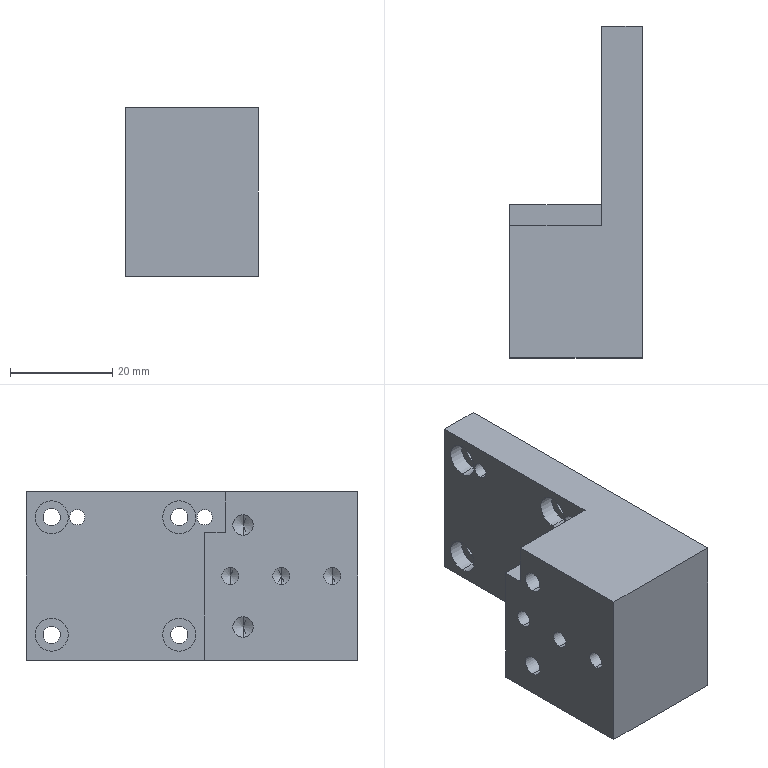Part | SolidWorks | features HoleWzd 4, LPattern 4, ICE 2, Extrusion 1 | 1 solid | 54 faces | box 26 x 65 x 33 mm | volume 33182 mm3 | cylinder 30 | plane 14 | cone 10 | commonest cylinder face diameters 3.4 x8 6.5 x8 3.3 x6 3 x4 4 x4
STEP:
#1=CARTESIAN_POINT('',(-8.,-10.,8.));
#2=VERTEX_POINT('',#1);
#3=CARTESIAN_POINT('',(-8.,-10.,12.));
#4=VERTEX_POINT('',#3);
#5=CARTESIAN_POINT('',(-8.,-10.,10.));
#6=DIRECTION('',(-1.,0.,0.));
#7=DIRECTION('',(0.,0.,1.));
#8=AXIS2_PLACEMENT_3D('',#5,#6,#7);
#9=CIRCLE('',#8,2.);
#10=EDGE_CURVE('',#2,#4,#9,.T.);
#11=ORIENTED_EDGE('',*,*,#10,.F.);
#12=CARTESIAN_POINT('',(-18.,-10.,8.));
#13=VERTEX_POINT('',#12);
#14=CARTESIAN_POINT('',(-18.,-10.,8.));
#15=DIRECTION('',(-1.,0.,0.));
#16=VECTOR('',#15,1000.);
#17=LINE('',#14,#16);
#18=EDGE_CURVE('',#2,#13,#17,.T.);
#19=ORIENTED_EDGE('',*,*,#18,.T.);
#20=CARTESIAN_POINT('',(-18.,-10.,12.));
#21=VERTEX_POINT('',#20);
#22=CARTESIAN_POINT('',(-18.,-10.,10.));
#23=DIRECTION('',(-1.,0.,0.));
#24=DIRECTION('',(0.,0.,1.));
#25=AXIS2_PLACEMENT_3D('',#22,#23,#24);
#26=CIRCLE('',#25,2.);
#27=EDGE_CURVE('',#13,#21,#26,.T.);
#28=ORIENTED_EDGE('',*,*,#27,.T.);
#29=CARTESIAN_POINT('',(-18.,-10.,12.));
#30=DIRECTION('',(-1.,0.,0.));
#31=VECTOR('',#30,1000.);
#32=LINE('',#29,#31);
#33=EDGE_CURVE('',#4,#21,#32,.T.);
#34=ORIENTED_EDGE('',*,*,#33,.F.);
#35=EDGE_LOOP('',(#11,#19,#28,#34));
#36=FACE_OUTER_BOUND('',#35,.T.);
#37=CARTESIAN_POINT('',(-18.,-10.,10.));
#38=DIRECTION('',(-1.,0.,0.));
#39=DIRECTION('',(0.,0.,1.));
#40=AXIS2_PLACEMENT_3D('',#37,#38,#39);
#41=CYLINDRICAL_SURFACE('',#40,2.);
#42=ADVANCED_FACE('',(#36),#41,.F.);
#43=CARTESIAN_POINT('',(-6.798,-10.,10.));
#44=VERTEX_POINT('',#43);
#45=CARTESIAN_POINT('',(-8.,-10.,12.));
#46=DIRECTION('',(-0.515,0.,0.8572));
#47=VECTOR('',#46,1000.);
#48=LINE('',#45,#47);
#49=EDGE_CURVE('',#44,#4,#48,.T.);
#50=ORIENTED_EDGE('',*,*,#49,.F.);
#51=CARTESIAN_POINT('',(-8.,-10.,8.));
#52=DIRECTION('',(-0.515,0.,-0.8572));
#53=VECTOR('',#52,1000.);
#54=LINE('',#51,#53);
#55=EDGE_CURVE('',#44,#2,#54,.T.);
#56=ORIENTED_EDGE('',*,*,#55,.T.);
#57=ORIENTED_EDGE('',*,*,#10,.T.);
#58=EDGE_LOOP('',(#50,#56,#57));
#59=FACE_OUTER_BOUND('',#58,.T.);
#60=CARTESIAN_POINT('',(-8.,-10.,10.));
#61=DIRECTION('',(-1.,0.,0.));
#62=DIRECTION('',(0.,0.,1.));
#63=AXIS2_PLACEMENT_3D('',#60,#61,#62);
#64=CONICAL_SURFACE('',#63,2.,1.03);
#65=ADVANCED_FACE('',(#59),#64,.F.);
#66=CARTESIAN_POINT('',(-8.,-10.,-12.));
#67=VERTEX_POINT('',#66);
#68=CARTESIAN_POINT('',(-8.,-10.,-8.));
#69=VERTEX_POINT('',#68);
#70=CARTESIAN_POINT('',(-8.,-10.,-10.));
#71=DIRECTION('',(-1.,0.,0.));
#72=DIRECTION('',(0.,0.,1.));
#73=AXIS2_PLACEMENT_3D('',#70,#71,#72);
#74=CIRCLE('',#73,2.);
#75=EDGE_CURVE('',#67,#69,#74,.T.);
#76=ORIENTED_EDGE('',*,*,#75,.F.);
#77=CARTESIAN_POINT('',(-18.,-10.,-12.));
#78=VERTEX_POINT('',#77);
#79=CARTESIAN_POINT('',(-18.,-10.,-12.));
#80=DIRECTION('',(-1.,0.,0.));
#81=VECTOR('',#80,1000.);
#82=LINE('',#79,#81);
#83=EDGE_CURVE('',#67,#78,#82,.T.);
#84=ORIENTED_EDGE('',*,*,#83,.T.);
#85=CARTESIAN_POINT('',(-18.,-10.,-8.));
#86=VERTEX_POINT('',#85);
#87=CARTESIAN_POINT('',(-18.,-10.,-10.));
#88=DIRECTION('',(-1.,0.,0.));
#89=DIRECTION('',(0.,0.,1.));
#90=AXIS2_PLACEMENT_3D('',#87,#88,#89);
#91=CIRCLE('',#90,2.);
#92=EDGE_CURVE('',#78,#86,#91,.T.);
#93=ORIENTED_EDGE('',*,*,#92,.T.);
#94=CARTESIAN_POINT('',(-18.,-10.,-8.));
#95=DIRECTION('',(-1.,0.,0.));
#96=VECTOR('',#95,1000.);
#97=LINE('',#94,#96);
#98=EDGE_CURVE('',#69,#86,#97,.T.);
#99=ORIENTED_EDGE('',*,*,#98,.F.);
#100=EDGE_LOOP('',(#76,#84,#93,#99));
#101=FACE_OUTER_BOUND('',#100,.T.);
#102=CARTESIAN_POINT('',(-18.,-10.,-10.));
#103=DIRECTION('',(-1.,0.,0.));
#104=DIRECTION('',(0.,0.,1.));
#105=AXIS2_PLACEMENT_3D('',#102,#103,#104);
#106=CYLINDRICAL_SURFACE('',#105,2.);
#107=ADVANCED_FACE('',(#101),#106,.F.);
#108=CARTESIAN_POINT('',(-6.798,-10.,-10.));
#109=VERTEX_POINT('',#108);
#110=CARTESIAN_POINT('',(-8.,-10.,-8.));
#111=DIRECTION('',(-0.515,0.,0.8572));
#112=VECTOR('',#111,1000.);
#113=LINE('',#110,#112);
#114=EDGE_CURVE('',#109,#69,#113,.T.);
#115=ORIENTED_EDGE('',*,*,#114,.F.);
#116=CARTESIAN_POINT('',(-8.,-10.,-12.));
#117=DIRECTION('',(-0.515,0.,-0.8572));
#118=VECTOR('',#117,1000.);
#119=LINE('',#116,#118);
#120=EDGE_CURVE('',#109,#67,#119,.T.);
#121=ORIENTED_EDGE('',*,*,#120,.T.);
#122=ORIENTED_EDGE('',*,*,#75,.T.);
#123=EDGE_LOOP('',(#115,#121,#122));
#124=FACE_OUTER_BOUND('',#123,.T.);
#125=CARTESIAN_POINT('',(-8.,-10.,-10.));
#126=DIRECTION('',(-1.,0.,0.));
#127=DIRECTION('',(0.,0.,1.));
#128=AXIS2_PLACEMENT_3D('',#125,#126,#127);
#129=CONICAL_SURFACE('',#128,2.,1.03);
#130=ADVANCED_FACE('',(#124),#129,.F.);
#131=CARTESIAN_POINT('',(8.,-2.5,10.));
#132=VERTEX_POINT('',#131);
#133=CARTESIAN_POINT('',(8.,-2.5,13.));
#134=VERTEX_POINT('',#133);
#135=CARTESIAN_POINT('',(8.,-2.5,11.5));
#136=DIRECTION('',(-1.,0.,0.));
#137=DIRECTION('',(0.,0.,1.));
#138=AXIS2_PLACEMENT_3D('',#135,#136,#137);
#139=CIRCLE('',#138,1.5);
#140=EDGE_CURVE('',#132,#134,#139,.T.);
#141=ORIENTED_EDGE('',*,*,#140,.F.);
#142=CARTESIAN_POINT('',(0.,-2.5,10.));
#143=VERTEX_POINT('',#142);
#144=CARTESIAN_POINT('',(0.,-2.5,10.));
#145=DIRECTION('',(-1.,0.,0.));
#146=VECTOR('',#145,1000.);
#147=LINE('',#144,#146);
#148=EDGE_CURVE('',#132,#143,#147,.T.);
#149=ORIENTED_EDGE('',*,*,#148,.T.);
#150=CARTESIAN_POINT('',(0.,-2.5,13.));
#151=VERTEX_POINT('',#150);
#152=CARTESIAN_POINT('',(0.,-2.5,11.5));
#153=DIRECTION('',(-1.,0.,0.));
#154=DIRECTION('',(0.,0.,1.));
#155=AXIS2_PLACEMENT_3D('',#152,#153,#154);
#156=CIRCLE('',#155,1.5);
#157=EDGE_CURVE('',#143,#151,#156,.T.);
#158=ORIENTED_EDGE('',*,*,#157,.T.);
#159=CARTESIAN_POINT('',(0.,-2.5,13.));
#160=DIRECTION('',(-1.,0.,0.));
#161=VECTOR('',#160,1000.);
#162=LINE('',#159,#161);
#163=EDGE_CURVE('',#134,#151,#162,.T.);
#164=ORIENTED_EDGE('',*,*,#163,.F.);
#165=EDGE_LOOP('',(#141,#149,#158,#164));
#166=FACE_OUTER_BOUND('',#165,.T.);
#167=CARTESIAN_POINT('',(0.,-2.5,11.5));
#168=DIRECTION('',(-1.,0.,0.));
#169=DIRECTION('',(0.,0.,1.));
#170=AXIS2_PLACEMENT_3D('',#167,#168,#169);
#171=CYLINDRICAL_SURFACE('',#170,1.5);
#172=ADVANCED_FACE('',(#166),#171,.F.);
#173=CARTESIAN_POINT('',(8.,22.5,10.));
#174=VERTEX_POINT('',#173);
#175=CARTESIAN_POINT('',(8.,22.5,13.));
#176=VERTEX_POINT('',#175);
#177=CARTESIAN_POINT('',(8.,22.5,11.5));
#178=DIRECTION('',(-1.,0.,0.));
#179=DIRECTION('',(0.,0.,1.));
#180=AXIS2_PLACEMENT_3D('',#177,#178,#179);
#181=CIRCLE('',#180,1.5);
#182=EDGE_CURVE('',#174,#176,#181,.T.);
#183=ORIENTED_EDGE('',*,*,#182,.F.);
#184=CARTESIAN_POINT('',(0.,22.5,10.));
#185=VERTEX_POINT('',#184);
#186=CARTESIAN_POINT('',(0.,22.5,10.));
#187=DIRECTION('',(-1.,0.,0.));
#188=VECTOR('',#187,1000.);
#189=LINE('',#186,#188);
#190=EDGE_CURVE('',#174,#185,#189,.T.);
#191=ORIENTED_EDGE('',*,*,#190,.T.);
#192=CARTESIAN_POINT('',(0.,22.5,13.));
#193=VERTEX_POINT('',#192);
#194=CARTESIAN_POINT('',(0.,22.5,11.5));
#195=DIRECTION('',(-1.,0.,0.));
#196=DIRECTION('',(0.,0.,1.));
#197=AXIS2_PLACEMENT_3D('',#194,#195,#196);
#198=CIRCLE('',#197,1.5);
#199=EDGE_CURVE('',#185,#193,#198,.T.);
#200=ORIENTED_EDGE('',*,*,#199,.T.);
#201=CARTESIAN_POINT('',(0.,22.5,13.));
#202=DIRECTION('',(-1.,0.,0.));
#203=VECTOR('',#202,1000.);
#204=LINE('',#201,#203);
#205=EDGE_CURVE('',#176,#193,#204,.T.);
#206=ORIENTED_EDGE('',*,*,#205,.F.);
#207=EDGE_LOOP('',(#183,#191,#200,#206));
#208=FACE_OUTER_BOUND('',#207,.T.);
#209=CARTESIAN_POINT('',(0.,22.5,11.5));
#210=DIRECTION('',(-1.,0.,0.));
#211=DIRECTION('',(0.,0.,1.));
#212=AXIS2_PLACEMENT_3D('',#209,#210,#211);
#213=CYLINDRICAL_SURFACE('',#212,1.5);
#214=ADVANCED_FACE('',(#208),#213,.F.);
#215=CARTESIAN_POINT('',(-6.909,-7.5,0.));
#216=VERTEX_POINT('',#215);
#217=CARTESIAN_POINT('',(-7.9,-7.5,1.65));
#218=VERTEX_POINT('',#217);
#219=CARTESIAN_POINT('',(-7.9,-7.5,1.65));
#220=DIRECTION('',(-0.515,0.,0.8572));
#221=VECTOR('',#220,1000.);
#222=LINE('',#219,#221);
#223=EDGE_CURVE('',#216,#218,#222,.T.);
#224=ORIENTED_EDGE('',*,*,#223,.F.);
#225=CARTESIAN_POINT('',(-7.9,-7.5,-1.65));
#226=VERTEX_POINT('',#225);
#227=CARTESIAN_POINT('',(-7.9,-7.5,-1.65));
#228=DIRECTION('',(-0.515,0.,-0.8572));
#229=VECTOR('',#228,1000.);
#230=LINE('',#227,#229);
#231=EDGE_CURVE('',#216,#226,#230,.T.);
#232=ORIENTED_EDGE('',*,*,#231,.T.);
#233=CARTESIAN_POINT('',(-7.9,-7.5,0.));
#234=DIRECTION('',(-1.,0.,0.));
#235=DIRECTION('',(0.,0.,1.));
#236=AXIS2_PLACEMENT_3D('',#233,#234,#235);
#237=CIRCLE('',#236,1.65);
#238=EDGE_CURVE('',#226,#218,#237,.T.);
#239=ORIENTED_EDGE('',*,*,#238,.T.);
#240=EDGE_LOOP('',(#224,#232,#239));
#241=FACE_OUTER_BOUND('',#240,.T.);
#242=CARTESIAN_POINT('',(-7.9,-7.5,0.));
#243=DIRECTION('',(-1.,0.,0.));
#244=DIRECTION('',(0.,0.,1.));
#245=AXIS2_PLACEMENT_3D('',#242,#243,#244);
#246=CONICAL_SURFACE('',#245,1.65,1.03);
#247=ADVANCED_FACE('',(#241),#246,.F.);
#248=ORIENTED_EDGE('',*,*,#238,.F.);
#249=CARTESIAN_POINT('',(-18.,-7.5,-1.65));
#250=VERTEX_POINT('',#249);
#251=CARTESIAN_POINT('',(-18.,-7.5,-1.65));
#252=DIRECTION('',(-1.,0.,0.));
#253=VECTOR('',#252,1000.);
#254=LINE('',#251,#253);
#255=EDGE_CURVE('',#226,#250,#254,.T.);
#256=ORIENTED_EDGE('',*,*,#255,.T.);
#257=CARTESIAN_POINT('',(-18.,-7.5,1.65));
#258=VERTEX_POINT('',#257);
#259=CARTESIAN_POINT('',(-18.,-7.5,0.));
#260=DIRECTION('',(-1.,0.,0.));
#261=DIRECTION('',(0.,0.,1.));
#262=AXIS2_PLACEMENT_3D('',#259,#260,#261);
#263=CIRCLE('',#262,1.65);
#264=EDGE_CURVE('',#250,#258,#263,.T.);
#265=ORIENTED_EDGE('',*,*,#264,.T.);
#266=CARTESIAN_POINT('',(-18.,-7.5,1.65));
#267=DIRECTION('',(-1.,0.,0.));
#268=VECTOR('',#267,1000.);
#269=LINE('',#266,#268);
#270=EDGE_CURVE('',#218,#258,#269,.T.);
#271=ORIENTED_EDGE('',*,*,#270,.F.);
#272=EDGE_LOOP('',(#248,#256,#265,#271));
#273=FACE_OUTER_BOUND('',#272,.T.);
#274=CARTESIAN_POINT('',(-18.,-7.5,0.));
#275=DIRECTION('',(-1.,0.,0.));
#276=DIRECTION('',(0.,0.,1.));
#277=AXIS2_PLACEMENT_3D('',#274,#275,#276);
#278=CYLINDRICAL_SURFACE('',#277,1.65);
#279=ADVANCED_FACE('',(#273),#278,.F.);
#280=CARTESIAN_POINT('',(-7.9,-17.5,-1.65));
#281=VERTEX_POINT('',#280);
#282=CARTESIAN_POINT('',(-7.9,-17.5,1.65));
#283=VERTEX_POINT('',#282);
#284=CARTESIAN_POINT('',(-7.9,-17.5,0.));
#285=DIRECTION('',(-1.,0.,0.));
#286=DIRECTION('',(0.,0.,1.));
#287=AXIS2_PLACEMENT_3D('',#284,#285,#286);
#288=CIRCLE('',#287,1.65);
#289=EDGE_CURVE('',#281,#283,#288,.T.);
#290=ORIENTED_EDGE('',*,*,#289,.F.);
#291=CARTESIAN_POINT('',(-18.,-17.5,-1.65));
#292=VERTEX_POINT('',#291);
#293=CARTESIAN_POINT('',(-18.,-17.5,-1.65));
#294=DIRECTION('',(-1.,0.,0.));
#295=VECTOR('',#294,1000.);
#296=LINE('',#293,#295);
#297=EDGE_CURVE('',#281,#292,#296,.T.);
#298=ORIENTED_EDGE('',*,*,#297,.T.);
#299=CARTESIAN_POINT('',(-18.,-17.5,1.65));
#300=VERTEX_POINT('',#299);
#301=CARTESIAN_POINT('',(-18.,-17.5,0.));
#302=DIRECTION('',(-1.,0.,0.));
#303=DIRECTION('',(0.,0.,1.));
#304=AXIS2_PLACEMENT_3D('',#301,#302,#303);
#305=CIRCLE('',#304,1.65);
#306=EDGE_CURVE('',#292,#300,#305,.T.);
#307=ORIENTED_EDGE('',*,*,#306,.T.);
#308=CARTESIAN_POINT('',(-18.,-17.5,1.65));
#309=DIRECTION('',(-1.,0.,0.));
#310=VECTOR('',#309,1000.);
#311=LINE('',#308,#310);
#312=EDGE_CURVE('',#283,#300,#311,.T.);
#313=ORIENTED_EDGE('',*,*,#312,.F.);
#314=EDGE_LOOP('',(#290,#298,#307,#313));
#315=FACE_OUTER_BOUND('',#314,.T.);
#316=CARTESIAN_POINT('',(-18.,-17.5,0.));
#317=DIRECTION('',(-1.,0.,0.));
#318=DIRECTION('',(0.,0.,1.));
#319=AXIS2_PLACEMENT_3D('',#316,#317,#318);
#320=CYLINDRICAL_SURFACE('',#319,1.65);
#321=ADVANCED_FACE('',(#315),#320,.F.);
#322=CARTESIAN_POINT('',(-6.909,-17.5,0.));
#323=VERTEX_POINT('',#322);
#324=CARTESIAN_POINT('',(-7.9,-17.5,1.65));
#325=DIRECTION('',(-0.515,0.,0.8572));
#326=VECTOR('',#325,1000.);
#327=LINE('',#324,#326);
#328=EDGE_CURVE('',#323,#283,#327,.T.);
#329=ORIENTED_EDGE('',*,*,#328,.F.);
#330=CARTESIAN_POINT('',(-7.9,-17.5,-1.65));
#331=DIRECTION('',(-0.515,0.,-0.8572));
#332=VECTOR('',#331,1000.);
#333=LINE('',#330,#332);
#334=EDGE_CURVE('',#323,#281,#333,.T.);
#335=ORIENTED_EDGE('',*,*,#334,.T.);
#336=ORIENTED_EDGE('',*,*,#289,.T.);
#337=EDGE_LOOP('',(#329,#335,#336));
#338=FACE_OUTER_BOUND('',#337,.T.);
#339=CARTESIAN_POINT('',(-7.9,-17.5,0.));
#340=DIRECTION('',(-1.,0.,0.));
#341=DIRECTION('',(0.,0.,1.));
#342=AXIS2_PLACEMENT_3D('',#339,#340,#341);
#343=CONICAL_SURFACE('',#342,1.65,1.03);
#344=ADVANCED_FACE('',(#338),#343,.F.);
#345=CARTESIAN_POINT('',(-7.9,-27.5,-1.65));
#346=VERTEX_POINT('',#345);
#347=CARTESIAN_POINT('',(-7.9,-27.5,1.65));
#348=VERTEX_POINT('',#347);
#349=CARTESIAN_POINT('',(-7.9,-27.5,0.));
#350=DIRECTION('',(-1.,0.,0.));
#351=DIRECTION('',(0.,0.,1.));
#352=AXIS2_PLACEMENT_3D('',#349,#350,#351);
#353=CIRCLE('',#352,1.65);
#354=EDGE_CURVE('',#346,#348,#353,.T.);
#355=ORIENTED_EDGE('',*,*,#354,.F.);
#356=CARTESIAN_POINT('',(-18.,-27.5,-1.65));
#357=VERTEX_POINT('',#356);
#358=CARTESIAN_POINT('',(-18.,-27.5,-1.65));
#359=DIRECTION('',(-1.,0.,0.));
#360=VECTOR('',#359,1000.);
#361=LINE('',#358,#360);
#362=EDGE_CURVE('',#346,#357,#361,.T.);
#363=ORIENTED_EDGE('',*,*,#362,.T.);
#364=CARTESIAN_POINT('',(-18.,-27.5,1.65));
#365=VERTEX_POINT('',#364);
#366=CARTESIAN_POINT('',(-18.,-27.5,0.));
#367=DIRECTION('',(-1.,0.,0.));
#368=DIRECTION('',(0.,0.,1.));
#369=AXIS2_PLACEMENT_3D('',#366,#367,#368);
#370=CIRCLE('',#369,1.65);
#371=EDGE_CURVE('',#357,#365,#370,.T.);
#372=ORIENTED_EDGE('',*,*,#371,.T.);
#373=CARTESIAN_POINT('',(-18.,-27.5,1.65));
#374=DIRECTION('',(-1.,0.,0.));
#375=VECTOR('',#374,1000.);
#376=LINE('',#373,#375);
#377=EDGE_CURVE('',#348,#365,#376,.T.);
#378=ORIENTED_EDGE('',*,*,#377,.F.);
#379=EDGE_LOOP('',(#355,#363,#372,#378));
#380=FACE_OUTER_BOUND('',#379,.T.);
#381=CARTESIAN_POINT('',(-18.,-27.5,0.));
#382=DIRECTION('',(-1.,0.,0.));
#383=DIRECTION('',(0.,0.,1.));
#384=AXIS2_PLACEMENT_3D('',#381,#382,#383);
#385=CYLINDRICAL_SURFACE('',#384,1.65);
#386=ADVANCED_FACE('',(#380),#385,.F.);
#387=CARTESIAN_POINT('',(-6.909,-27.5,0.));
#388=VERTEX_POINT('',#387);
#389=CARTESIAN_POINT('',(-7.9,-27.5,1.65));
#390=DIRECTION('',(-0.515,0.,0.8572));
#391=VECTOR('',#390,1000.);
#392=LINE('',#389,#391);
#393=EDGE_CURVE('',#388,#348,#392,.T.);
#394=ORIENTED_EDGE('',*,*,#393,.F.);
#395=CARTESIAN_POINT('',(-7.9,-27.5,-1.65));
#396=DIRECTION('',(-0.515,0.,-0.8572));
#397=VECTOR('',#396,1000.);
#398=LINE('',#395,#397);
#399=EDGE_CURVE('',#388,#346,#398,.T.);
#400=ORIENTED_EDGE('',*,*,#399,.T.);
#401=ORIENTED_EDGE('',*,*,#354,.T.);
#402=EDGE_LOOP('',(#394,#400,#401));
#403=FACE_OUTER_BOUND('',#402,.T.);
#404=CARTESIAN_POINT('',(-7.9,-27.5,0.));
#405=DIRECTION('',(-1.,0.,0.));
#406=DIRECTION('',(0.,0.,1.));
#407=AXIS2_PLACEMENT_3D('',#404,#405,#406);
#408=CONICAL_SURFACE('',#407,1.65,1.03);
#409=ADVANCED_FACE('',(#403),#408,.F.);
#410=CARTESIAN_POINT('',(8.,2.5,9.8));
#411=VERTEX_POINT('',#410);
#412=CARTESIAN_POINT('',(8.,2.5,13.2));
#413=VERTEX_POINT('',#412);
#414=CARTESIAN_POINT('',(8.,2.5,11.5));
#415=DIRECTION('',(-1.,0.,0.));
#416=DIRECTION('',(0.,0.,1.));
#417=AXIS2_PLACEMENT_3D('',#414,#415,#416);
#418=CIRCLE('',#417,1.7);
#419=EDGE_CURVE('',#411,#413,#418,.T.);
#420=ORIENTED_EDGE('',*,*,#419,.F.);
#421=CARTESIAN_POINT('',(3.,2.5,9.8));
#422=VERTEX_POINT('',#421);
#423=CARTESIAN_POINT('',(0.,2.5,9.8));
#424=DIRECTION('',(-1.,0.,0.));
#425=VECTOR('',#424,1000.);
#426=LINE('',#423,#425);
#427=EDGE_CURVE('',#411,#422,#426,.T.);
#428=ORIENTED_EDGE('',*,*,#427,.T.);
#429=CARTESIAN_POINT('',(3.,2.5,13.2));
#430=VERTEX_POINT('',#429);
#431=CARTESIAN_POINT('',(3.,2.5,11.5));
#432=DIRECTION('',(-1.,0.,0.));
#433=DIRECTION('',(0.,0.,1.));
#434=AXIS2_PLACEMENT_3D('',#431,#432,#433);
#435=CIRCLE('',#434,1.7);
#436=EDGE_CURVE('',#422,#430,#435,.T.);
#437=ORIENTED_EDGE('',*,*,#436,.T.);
#438=CARTESIAN_POINT('',(0.,2.5,13.2));
#439=DIRECTION('',(-1.,0.,0.));
#440=VECTOR('',#439,1000.);
#441=LINE('',#438,#440);
#442=EDGE_CURVE('',#413,#430,#441,.T.);
#443=ORIENTED_EDGE('',*,*,#442,.F.);
#444=EDGE_LOOP('',(#420,#428,#437,#443));
#445=FACE_OUTER_BOUND('',#444,.T.);
#446=CARTESIAN_POINT('',(0.,2.5,11.5));
#447=DIRECTION('',(-1.,0.,0.));
#448=DIRECTION('',(0.,0.,1.));
#449=AXIS2_PLACEMENT_3D('',#446,#447,#448);
#450=CYLINDRICAL_SURFACE('',#449,1.7);
#451=ADVANCED_FACE('',(#445),#450,.F.);
#452=CARTESIAN_POINT('',(3.,2.5,8.25));
#453=VERTEX_POINT('',#452);
#454=CARTESIAN_POINT('',(3.,2.5,14.75));
#455=VERTEX_POINT('',#454);
#456=CARTESIAN_POINT('',(3.,2.5,11.5));
#457=DIRECTION('',(-1.,0.,0.));
#458=DIRECTION('',(0.,0.,1.));
#459=AXIS2_PLACEMENT_3D('',#456,#457,#458);
#460=CIRCLE('',#459,3.25);
#461=EDGE_CURVE('',#453,#455,#460,.T.);
#462=ORIENTED_EDGE('',*,*,#461,.F.);
#463=CARTESIAN_POINT('',(0.,2.5,8.25));
#464=VERTEX_POINT('',#463);
#465=CARTESIAN_POINT('',(0.,2.5,8.25));
#466=DIRECTION('',(-1.,0.,0.));
#467=VECTOR('',#466,1000.);
#468=LINE('',#465,#467);
#469=EDGE_CURVE('',#453,#464,#468,.T.);
#470=ORIENTED_EDGE('',*,*,#469,.T.);
#471=CARTESIAN_POINT('',(0.,2.5,14.75));
#472=VERTEX_POINT('',#471);
#473=CARTESIAN_POINT('',(0.,2.5,11.5));
#474=DIRECTION('',(-1.,0.,0.));
#475=DIRECTION('',(0.,0.,1.));
#476=AXIS2_PLACEMENT_3D('',#473,#474,#475);
#477=CIRCLE('',#476,3.25);
#478=EDGE_CURVE('',#464,#472,#477,.T.);
#479=ORIENTED_EDGE('',*,*,#478,.T.);
#480=CARTESIAN_POINT('',(0.,2.5,14.75));
#481=DIRECTION('',(-1.,0.,0.));
#482=VECTOR('',#481,1000.);
#483=LINE('',#480,#482);
#484=EDGE_CURVE('',#455,#472,#483,.T.);
#485=ORIENTED_EDGE('',*,*,#484,.F.);
#486=EDGE_LOOP('',(#462,#470,#479,#485));
#487=FACE_OUTER_BOUND('',#486,.T.);
#488=CARTESIAN_POINT('',(0.,2.5,11.5));
#489=DIRECTION('',(-1.,0.,0.));
#490=DIRECTION('',(0.,0.,1.));
#491=AXIS2_PLACEMENT_3D('',#488,#489,#490);
#492=CYLINDRICAL_SURFACE('',#491,3.25);
#493=ADVANCED_FACE('',(#487),#492,.F.);
#494=CARTESIAN_POINT('',(8.,2.5,-13.2));
#495=VERTEX_POINT('',#494);
#496=CARTESIAN_POINT('',(8.,2.5,-9.8));
#497=VERTEX_POINT('',#496);
#498=CARTESIAN_POINT('',(8.,2.5,-11.5));
#499=DIRECTION('',(-1.,0.,0.));
#500=DIRECTION('',(0.,0.,1.));
#501=AXIS2_PLACEMENT_3D('',#498,#499,#500);
#502=CIRCLE('',#501,1.7);
#503=EDGE_CURVE('',#495,#497,#502,.T.);
#504=ORIENTED_EDGE('',*,*,#503,.F.);
#505=CARTESIAN_POINT('',(3.,2.5,-13.2));
#506=VERTEX_POINT('',#505);
#507=CARTESIAN_POINT('',(0.,2.5,-13.2));
#508=DIRECTION('',(-1.,0.,0.));
#509=VECTOR('',#508,1000.);
#510=LINE('',#507,#509);
#511=EDGE_CURVE('',#495,#506,#510,.T.);
#512=ORIENTED_EDGE('',*,*,#511,.T.);
#513=CARTESIAN_POINT('',(3.,2.5,-9.8));
#514=VERTEX_POINT('',#513);
#515=CARTESIAN_POINT('',(3.,2.5,-11.5));
#516=DIRECTION('',(-1.,0.,0.));
#517=DIRECTION('',(0.,0.,1.));
#518=AXIS2_PLACEMENT_3D('',#515,#516,#517);
#519=CIRCLE('',#518,1.7);
#520=EDGE_CURVE('',#506,#514,#519,.T.);
#521=ORIENTED_EDGE('',*,*,#520,.T.);
#522=CARTESIAN_POINT('',(0.,2.5,-9.8));
#523=DIRECTION('',(-1.,0.,0.));
#524=VECTOR('',#523,1000.);
#525=LINE('',#522,#524);
#526=EDGE_CURVE('',#497,#514,#525,.T.);
#527=ORIENTED_EDGE('',*,*,#526,.F.);
#528=EDGE_LOOP('',(#504,#512,#521,#527));
#529=FACE_OUTER_BOUND('',#528,.T.);
#530=CARTESIAN_POINT('',(0.,2.5,-11.5));
#531=DIRECTION('',(-1.,0.,0.));
#532=DIRECTION('',(0.,0.,1.));
#533=AXIS2_PLACEMENT_3D('',#530,#531,#532);
#534=CYLINDRICAL_SURFACE('',#533,1.7);
#535=ADVANCED_FACE('',(#529),#534,.F.);
#536=CARTESIAN_POINT('',(3.,2.5,-14.75));
#537=VERTEX_POINT('',#536);
#538=CARTESIAN_POINT('',(3.,2.5,-8.25));
#539=VERTEX_POINT('',#538);
#540=CARTESIAN_POINT('',(3.,2.5,-11.5));
#541=DIRECTION('',(-1.,0.,0.));
#542=DIRECTION('',(0.,0.,1.));
#543=AXIS2_PLACEMENT_3D('',#540,#541,#542);
#544=CIRCLE('',#543,3.25);
#545=EDGE_CURVE('',#537,#539,#544,.T.);
#546=ORIENTED_EDGE('',*,*,#545,.F.);
#547=CARTESIAN_POINT('',(0.,2.5,-14.75));
#548=VERTEX_POINT('',#547);
#549=CARTESIAN_POINT('',(0.,2.5,-14.75));
#550=DIRECTION('',(-1.,0.,0.));
#551=VECTOR('',#550,1000.);
#552=LINE('',#549,#551);
#553=EDGE_CURVE('',#537,#548,#552,.T.);
#554=ORIENTED_EDGE('',*,*,#553,.T.);
#555=CARTESIAN_POINT('',(0.,2.5,-8.25));
#556=VERTEX_POINT('',#555);
#557=CARTESIAN_POINT('',(0.,2.5,-11.5));
#558=DIRECTION('',(-1.,0.,0.));
#559=DIRECTION('',(0.,0.,1.));
#560=AXIS2_PLACEMENT_3D('',#557,#558,#559);
#561=CIRCLE('',#560,3.25);
#562=EDGE_CURVE('',#548,#556,#561,.T.);
#563=ORIENTED_EDGE('',*,*,#562,.T.);
#564=CARTESIAN_POINT('',(0.,2.5,-8.25));
#565=DIRECTION('',(-1.,0.,0.));
#566=VECTOR('',#565,1000.);
#567=LINE('',#564,#566);
#568=EDGE_CURVE('',#539,#556,#567,.T.);
#569=ORIENTED_EDGE('',*,*,#568,.F.);
#570=EDGE_LOOP('',(#546,#554,#563,#569));
#571=FACE_OUTER_BOUND('',#570,.T.);
#572=CARTESIAN_POINT('',(0.,2.5,-11.5));
#573=DIRECTION('',(-1.,0.,0.));
#574=DIRECTION('',(0.,0.,1.));
#575=AXIS2_PLACEMENT_3D('',#572,#573,#574);
#576=CYLINDRICAL_SURFACE('',#575,3.25);
#577=ADVANCED_FACE('',(#571),#576,.F.);
#578=CARTESIAN_POINT('',(3.,27.5,8.25));
#579=VERTEX_POINT('',#578);
#580=CARTESIAN_POINT('',(3.,27.5,14.75));
#581=VERTEX_POINT('',#580);
#582=CARTESIAN_POINT('',(3.,27.5,11.5));
#583=DIRECTION('',(-1.,0.,0.));
#584=DIRECTION('',(0.,0.,1.));
#585=AXIS2_PLACEMENT_3D('',#582,#583,#584);
#586=CIRCLE('',#585,3.25);
#587=EDGE_CURVE('',#579,#581,#586,.T.);
#588=ORIENTED_EDGE('',*,*,#587,.F.);
#589=CARTESIAN_POINT('',(0.,27.5,8.25));
#590=VERTEX_POINT('',#589);
#591=CARTESIAN_POINT('',(0.,27.5,8.25));
#592=DIRECTION('',(-1.,0.,0.));
#593=VECTOR('',#592,1000.);
#594=LINE('',#591,#593);
#595=EDGE_CURVE('',#579,#590,#594,.T.);
#596=ORIENTED_EDGE('',*,*,#595,.T.);
#597=CARTESIAN_POINT('',(0.,27.5,14.75));
#598=VERTEX_POINT('',#597);
#599=CARTESIAN_POINT('',(0.,27.5,11.5));
#600=DIRECTION('',(-1.,0.,0.));
#601=DIRECTION('',(0.,0.,1.));
#602=AXIS2_PLACEMENT_3D('',#599,#600,#601);
#603=CIRCLE('',#602,3.25);
#604=EDGE_CURVE('',#590,#598,#603,.T.);
#605=ORIENTED_EDGE('',*,*,#604,.T.);
#606=CARTESIAN_POINT('',(0.,27.5,14.75));
#607=DIRECTION('',(-1.,0.,0.));
#608=VECTOR('',#607,1000.);
#609=LINE('',#606,#608);
#610=EDGE_CURVE('',#581,#598,#609,.T.);
#611=ORIENTED_EDGE('',*,*,#610,.F.);
#612=EDGE_LOOP('',(#588,#596,#605,#611));
#613=FACE_OUTER_BOUND('',#612,.T.);
#614=CARTESIAN_POINT('',(0.,27.5,11.5));
#615=DIRECTION('',(-1.,0.,0.));
#616=DIRECTION('',(0.,0.,1.));
#617=AXIS2_PLACEMENT_3D('',#614,#615,#616);
#618=CYLINDRICAL_SURFACE('',#617,3.25);
#619=ADVANCED_FACE('',(#613),#618,.F.);
#620=CARTESIAN_POINT('',(8.,27.5,9.8));
#621=VERTEX_POINT('',#620);
#622=CARTESIAN_POINT('',(8.,27.5,13.2));
#623=VERTEX_POINT('',#622);
#624=CARTESIAN_POINT('',(8.,27.5,11.5));
#625=DIRECTION('',(-1.,0.,0.));
#626=DIRECTION('',(0.,0.,1.));
#627=AXIS2_PLACEMENT_3D('',#624,#625,#626);
#628=CIRCLE('',#627,1.7);
#629=EDGE_CURVE('',#621,#623,#628,.T.);
#630=ORIENTED_EDGE('',*,*,#629,.F.);
#631=CARTESIAN_POINT('',(3.,27.5,9.8));
#632=VERTEX_POINT('',#631);
#633=CARTESIAN_POINT('',(0.,27.5,9.8));
#634=DIRECTION('',(-1.,0.,0.));
#635=VECTOR('',#634,1000.);
#636=LINE('',#633,#635);
#637=EDGE_CURVE('',#621,#632,#636,.T.);
#638=ORIENTED_EDGE('',*,*,#637,.T.);
#639=CARTESIAN_POINT('',(3.,27.5,13.2));
#640=VERTEX_POINT('',#639);
#641=CARTESIAN_POINT('',(3.,27.5,11.5));
#642=DIRECTION('',(-1.,0.,0.));
#643=DIRECTION('',(0.,0.,1.));
#644=AXIS2_PLACEMENT_3D('',#641,#642,#643);
#645=CIRCLE('',#644,1.7);
#646=EDGE_CURVE('',#632,#640,#645,.T.);
#647=ORIENTED_EDGE('',*,*,#646,.T.);
#648=CARTESIAN_POINT('',(0.,27.5,13.2));
#649=DIRECTION('',(-1.,0.,0.));
#650=VECTOR('',#649,1000.);
#651=LINE('',#648,#650);
#652=EDGE_CURVE('',#623,#640,#651,.T.);
#653=ORIENTED_EDGE('',*,*,#652,.F.);
#654=EDGE_LOOP('',(#630,#638,#647,#653));
#655=FACE_OUTER_BOUND('',#654,.T.);
#656=CARTESIAN_POINT('',(0.,27.5,11.5));
#657=DIRECTION('',(-1.,0.,0.));
#658=DIRECTION('',(0.,0.,1.));
#659=AXIS2_PLACEMENT_3D('',#656,#657,#658);
#660=CYLINDRICAL_SURFACE('',#659,1.7);
#661=ADVANCED_FACE('',(#655),#660,.F.);
#662=CARTESIAN_POINT('',(3.,27.5,-14.75));
#663=VERTEX_POINT('',#662);
#664=CARTESIAN_POINT('',(3.,27.5,-8.25));
#665=VERTEX_POINT('',#664);
#666=CARTESIAN_POINT('',(3.,27.5,-11.5));
#667=DIRECTION('',(-1.,0.,0.));
#668=DIRECTION('',(0.,0.,1.));
#669=AXIS2_PLACEMENT_3D('',#666,#667,#668);
#670=CIRCLE('',#669,3.25);
#671=EDGE_CURVE('',#663,#665,#670,.T.);
#672=ORIENTED_EDGE('',*,*,#671,.F.);
#673=CARTESIAN_POINT('',(0.,27.5,-14.75));
#674=VERTEX_POINT('',#673);
#675=CARTESIAN_POINT('',(0.,27.5,-14.75));
#676=DIRECTION('',(-1.,0.,0.));
#677=VECTOR('',#676,1000.);
#678=LINE('',#675,#677);
#679=EDGE_CURVE('',#663,#674,#678,.T.);
#680=ORIENTED_EDGE('',*,*,#679,.T.);
#681=CARTESIAN_POINT('',(0.,27.5,-8.25));
#682=VERTEX_POINT('',#681);
#683=CARTESIAN_POINT('',(0.,27.5,-11.5));
#684=DIRECTION('',(-1.,0.,0.));
#685=DIRECTION('',(0.,0.,1.));
#686=AXIS2_PLACEMENT_3D('',#683,#684,#685);
#687=CIRCLE('',#686,3.25);
#688=EDGE_CURVE('',#674,#682,#687,.T.);
#689=ORIENTED_EDGE('',*,*,#688,.T.);
#690=CARTESIAN_POINT('',(0.,27.5,-8.25));
#691=DIRECTION('',(-1.,0.,0.));
#692=VECTOR('',#691,1000.);
#693=LINE('',#690,#692);
#694=EDGE_CURVE('',#665,#682,#693,.T.);
#695=ORIENTED_EDGE('',*,*,#694,.F.);
#696=EDGE_LOOP('',(#672,#680,#689,#695));
#697=FACE_OUTER_BOUND('',#696,.T.);
#698=CARTESIAN_POINT('',(0.,27.5,-11.5));
#699=DIRECTION('',(-1.,0.,0.));
#700=DIRECTION('',(0.,0.,1.));
#701=AXIS2_PLACEMENT_3D('',#698,#699,#700);
#702=CYLINDRICAL_SURFACE('',#701,3.25);
#703=ADVANCED_FACE('',(#697),#702,.F.);
#704=CARTESIAN_POINT('',(8.,27.5,-13.2));
#705=VERTEX_POINT('',#704);
#706=CARTESIAN_POINT('',(8.,27.5,-9.8));
#707=VERTEX_POINT('',#706);
#708=CARTESIAN_POINT('',(8.,27.5,-11.5));
#709=DIRECTION('',(-1.,0.,0.));
#710=DIRECTION('',(0.,0.,1.));
#711=AXIS2_PLACEMENT_3D('',#708,#709,#710);
#712=CIRCLE('',#711,1.7);
#713=EDGE_CURVE('',#705,#707,#712,.T.);
#714=ORIENTED_EDGE('',*,*,#713,.F.);
#715=CARTESIAN_POINT('',(3.,27.5,-13.2));
#716=VERTEX_POINT('',#715);
#717=CARTESIAN_POINT('',(0.,27.5,-13.2));
#718=DIRECTION('',(-1.,0.,0.));
#719=VECTOR('',#718,1000.);
#720=LINE('',#717,#719);
#721=EDGE_CURVE('',#705,#716,#720,.T.);
#722=ORIENTED_EDGE('',*,*,#721,.T.);
#723=CARTESIAN_POINT('',(3.,27.5,-9.8));
#724=VERTEX_POINT('',#723);
#725=CARTESIAN_POINT('',(3.,27.5,-11.5));
#726=DIRECTION('',(-1.,0.,0.));
#727=DIRECTION('',(0.,0.,1.));
#728=AXIS2_PLACEMENT_3D('',#725,#726,#727);
#729=CIRCLE('',#728,1.7);
#730=EDGE_CURVE('',#716,#724,#729,.T.);
#731=ORIENTED_EDGE('',*,*,#730,.T.);
#732=CARTESIAN_POINT('',(0.,27.5,-9.8));
#733=DIRECTION('',(-1.,0.,0.));
#734=VECTOR('',#733,1000.);
#735=LINE('',#732,#734);
#736=EDGE_CURVE('',#707,#724,#735,.T.);
#737=ORIENTED_EDGE('',*,*,#736,.F.);
#738=EDGE_LOOP('',(#714,#722,#731,#737));
#739=FACE_OUTER_BOUND('',#738,.T.);
#740=CARTESIAN_POINT('',(0.,27.5,-11.5));
#741=DIRECTION('',(-1.,0.,0.));
#742=DIRECTION('',(0.,0.,1.));
#743=AXIS2_PLACEMENT_3D('',#740,#741,#742);
#744=CYLINDRICAL_SURFACE('',#743,1.7);
#745=ADVANCED_FACE('',(#739),#744,.F.);
#746=CARTESIAN_POINT('',(8.,-32.5,-16.5));
#747=VERTEX_POINT('',#746);
#748=CARTESIAN_POINT('',(-18.,-32.5,-16.5));
#749=VERTEX_POINT('',#748);
#750=CARTESIAN_POINT('',(8.,-32.5,-16.5));
#751=DIRECTION('',(-1.,0.,0.));
#752=VECTOR('',#751,1000.);
#753=LINE('',#750,#752);
#754=EDGE_CURVE('',#747,#749,#753,.T.);
#755=ORIENTED_EDGE('',*,*,#754,.T.);
#756=CARTESIAN_POINT('',(-18.,-2.5,-16.5));
#757=VERTEX_POINT('',#756);
#758=CARTESIAN_POINT('',(-18.,-32.5,-16.5));
#759=DIRECTION('',(0.,-1.,0.));
#760=VECTOR('',#759,1000.);
#761=LINE('',#758,#760);
#762=EDGE_CURVE('',#757,#749,#761,.T.);
#763=ORIENTED_EDGE('',*,*,#762,.F.);
#764=CARTESIAN_POINT('',(0.,-2.5,-16.5));
#765=VERTEX_POINT('',#764);
#766=CARTESIAN_POINT('',(-18.,-2.5,-16.5));
#767=DIRECTION('',(1.,0.,0.));
#768=VECTOR('',#767,1000.);
#769=LINE('',#766,#768);
#770=EDGE_CURVE('',#757,#765,#769,.T.);
#771=ORIENTED_EDGE('',*,*,#770,.T.);
#772=CARTESIAN_POINT('',(0.,32.5,-16.5));
#773=VERTEX_POINT('',#772);
#774=CARTESIAN_POINT('',(0.,-32.5,-16.5));
#775=DIRECTION('',(0.,1.,0.));
#776=VECTOR('',#775,1000.);
#777=LINE('',#774,#776);
#778=EDGE_CURVE('',#765,#773,#777,.T.);
#779=ORIENTED_EDGE('',*,*,#778,.T.);
#780=CARTESIAN_POINT('',(8.,32.5,-16.5));
#781=VERTEX_POINT('',#780);
#782=CARTESIAN_POINT('',(8.,32.5,-16.5));
#783=DIRECTION('',(-1.,0.,0.));
#784=VECTOR('',#783,1000.);
#785=LINE('',#782,#784);
#786=EDGE_CURVE('',#781,#773,#785,.T.);
#787=ORIENTED_EDGE('',*,*,#786,.F.);
#788=CARTESIAN_POINT('',(8.,-32.5,-16.5));
#789=DIRECTION('',(0.,1.,0.));
#790=VECTOR('',#789,1000.);
#791=LINE('',#788,#790);
#792=EDGE_CURVE('',#747,#781,#791,.T.);
#793=ORIENTED_EDGE('',*,*,#792,.F.);
#794=EDGE_LOOP('',(#755,#763,#771,#779,#787,#793));
#795=FACE_OUTER_BOUND('',#794,.T.);
#796=CARTESIAN_POINT('',(8.,-32.5,-16.5));
#797=DIRECTION('',(0.,0.,1.));
#798=DIRECTION('',(1.,0.,0.));
#799=AXIS2_PLACEMENT_3D('',#796,#797,#798);
#800=PLANE('',#799);
#801=ADVANCED_FACE('',(#795),#800,.F.);
#802=CARTESIAN_POINT('',(0.,32.5,16.5));
#803=VERTEX_POINT('',#802);
#804=CARTESIAN_POINT('',(0.,32.5,16.5));
#805=DIRECTION('',(0.,0.,1.));
#806=VECTOR('',#805,1000.);
#807=LINE('',#804,#806);
#808=EDGE_CURVE('',#773,#803,#807,.T.);
#809=ORIENTED_EDGE('',*,*,#808,.T.);
#810=CARTESIAN_POINT('',(8.,32.5,16.5));
#811=VERTEX_POINT('',#810);
#812=CARTESIAN_POINT('',(8.,32.5,16.5));
#813=DIRECTION('',(-1.,0.,0.));
#814=VECTOR('',#813,1000.);
#815=LINE('',#812,#814);
#816=EDGE_CURVE('',#811,#803,#815,.T.);
#817=ORIENTED_EDGE('',*,*,#816,.F.);
#818=CARTESIAN_POINT('',(8.,32.5,16.5));
#819=DIRECTION('',(0.,0.,1.));
#820=VECTOR('',#819,1000.);
#821=LINE('',#818,#820);
#822=EDGE_CURVE('',#781,#811,#821,.T.);
#823=ORIENTED_EDGE('',*,*,#822,.F.);
#824=ORIENTED_EDGE('',*,*,#786,.T.);
#825=EDGE_LOOP('',(#809,#817,#823,#824));
#826=FACE_OUTER_BOUND('',#825,.T.);
#827=CARTESIAN_POINT('',(8.,32.5,16.5));
#828=DIRECTION('',(0.,-1.,0.));
#829=DIRECTION('',(0.,0.,-1.));
#830=AXIS2_PLACEMENT_3D('',#827,#828,#829);
#831=PLANE('',#830);
#832=ADVANCED_FACE('',(#826),#831,.F.);
#833=CARTESIAN_POINT('',(0.,-6.5,16.5));
#834=VERTEX_POINT('',#833);
#835=CARTESIAN_POINT('',(0.,-32.5,16.5));
#836=DIRECTION('',(0.,-1.,0.));
#837=VECTOR('',#836,1000.);
#838=LINE('',#835,#837);
#839=EDGE_CURVE('',#803,#834,#838,.T.);
#840=ORIENTED_EDGE('',*,*,#839,.T.);
#841=CARTESIAN_POINT('',(-18.,-6.5,16.5));
#842=VERTEX_POINT('',#841);
#843=CARTESIAN_POINT('',(8.944,-6.5,16.5));
#844=DIRECTION('',(-1.,0.,0.));
#845=VECTOR('',#844,1000.);
#846=LINE('',#843,#845);
#847=EDGE_CURVE('',#834,#842,#846,.T.);
#848=ORIENTED_EDGE('',*,*,#847,.T.);
#849=CARTESIAN_POINT('',(-18.,-32.5,16.5));
#850=VERTEX_POINT('',#849);
#851=CARTESIAN_POINT('',(-18.,-32.5,16.5));
#852=DIRECTION('',(0.,1.,0.));
#853=VECTOR('',#852,1000.);
#854=LINE('',#851,#853);
#855=EDGE_CURVE('',#850,#842,#854,.T.);
#856=ORIENTED_EDGE('',*,*,#855,.F.);
#857=CARTESIAN_POINT('',(8.,-32.5,16.5));
#858=VERTEX_POINT('',#857);
#859=CARTESIAN_POINT('',(8.,-32.5,16.5));
#860=DIRECTION('',(-1.,0.,0.));
#861=VECTOR('',#860,1000.);
#862=LINE('',#859,#861);
#863=EDGE_CURVE('',#858,#850,#862,.T.);
#864=ORIENTED_EDGE('',*,*,#863,.F.);
#865=CARTESIAN_POINT('',(8.,-32.5,16.5));
#866=DIRECTION('',(0.,-1.,0.));
#867=VECTOR('',#866,1000.);
#868=LINE('',#865,#867);
#869=EDGE_CURVE('',#811,#858,#868,.T.);
#870=ORIENTED_EDGE('',*,*,#869,.F.);
#871=ORIENTED_EDGE('',*,*,#816,.T.);
#872=EDGE_LOOP('',(#840,#848,#856,#864,#870,#871));
#873=FACE_OUTER_BOUND('',#872,.T.);
#874=CARTESIAN_POINT('',(8.,-32.5,16.5));
#875=DIRECTION('',(0.,0.,-1.));
#876=DIRECTION('',(-1.,0.,0.));
#877=AXIS2_PLACEMENT_3D('',#874,#875,#876);
#878=PLANE('',#877);
#879=ADVANCED_FACE('',(#873),#878,.F.);
#880=ORIENTED_EDGE('',*,*,#863,.T.);
#881=CARTESIAN_POINT('',(-18.,-32.5,-16.5));
#882=DIRECTION('',(0.,0.,1.));
#883=VECTOR('',#882,1000.);
#884=LINE('',#881,#883);
#885=EDGE_CURVE('',#749,#850,#884,.T.);
#886=ORIENTED_EDGE('',*,*,#885,.F.);
#887=ORIENTED_EDGE('',*,*,#754,.F.);
#888=CARTESIAN_POINT('',(8.,-32.5,16.5));
#889=DIRECTION('',(0.,0.,-1.));
#890=VECTOR('',#889,1000.);
#891=LINE('',#888,#890);
#892=EDGE_CURVE('',#858,#747,#891,.T.);
#893=ORIENTED_EDGE('',*,*,#892,.F.);
#894=EDGE_LOOP('',(#880,#886,#887,#893));
#895=FACE_OUTER_BOUND('',#894,.T.);
#896=CARTESIAN_POINT('',(8.,-32.5,16.5));
#897=DIRECTION('',(0.,1.,0.));
#898=DIRECTION('',(0.,0.,1.));
#899=AXIS2_PLACEMENT_3D('',#896,#897,#898);
#900=PLANE('',#899);
#901=ADVANCED_FACE('',(#895),#900,.F.);
#902=CARTESIAN_POINT('',(8.,-2.5,11.5));
#903=DIRECTION('',(-1.,0.,0.));
#904=DIRECTION('',(0.,0.,1.));
#905=AXIS2_PLACEMENT_3D('',#902,#903,#904);
#906=CIRCLE('',#905,1.5);
#907=EDGE_CURVE('',#134,#132,#906,.T.);
#908=ORIENTED_EDGE('',*,*,#907,.T.);
#909=ORIENTED_EDGE('',*,*,#140,.T.);
#910=EDGE_LOOP('',(#908,#909));
#911=FACE_BOUND('',#910,.T.);
#912=CARTESIAN_POINT('',(8.,22.5,11.5));
#913=DIRECTION('',(-1.,0.,0.));
#914=DIRECTION('',(0.,0.,1.));
#915=AXIS2_PLACEMENT_3D('',#912,#913,#914);
#916=CIRCLE('',#915,1.5);
#917=EDGE_CURVE('',#176,#174,#916,.T.);
#918=ORIENTED_EDGE('',*,*,#917,.T.);
#919=ORIENTED_EDGE('',*,*,#182,.T.);
#920=EDGE_LOOP('',(#918,#919));
#921=FACE_BOUND('',#920,.T.);
#922=CARTESIAN_POINT('',(8.,27.5,11.5));
#923=DIRECTION('',(-1.,0.,0.));
#924=DIRECTION('',(0.,0.,1.));
#925=AXIS2_PLACEMENT_3D('',#922,#923,#924);
#926=CIRCLE('',#925,1.7);
#927=EDGE_CURVE('',#623,#621,#926,.T.);
#928=ORIENTED_EDGE('',*,*,#927,.T.);
#929=ORIENTED_EDGE('',*,*,#629,.T.);
#930=EDGE_LOOP('',(#928,#929));
#931=FACE_BOUND('',#930,.T.);
#932=CARTESIAN_POINT('',(8.,27.5,-11.5));
#933=DIRECTION('',(-1.,0.,0.));
#934=DIRECTION('',(0.,0.,1.));
#935=AXIS2_PLACEMENT_3D('',#932,#933,#934);
#936=CIRCLE('',#935,1.7);
#937=EDGE_CURVE('',#707,#705,#936,.T.);
#938=ORIENTED_EDGE('',*,*,#937,.T.);
#939=ORIENTED_EDGE('',*,*,#713,.T.);
#940=EDGE_LOOP('',(#938,#939));
#941=FACE_BOUND('',#940,.T.);
#942=ORIENTED_EDGE('',*,*,#792,.T.);
#943=ORIENTED_EDGE('',*,*,#822,.T.);
#944=ORIENTED_EDGE('',*,*,#869,.T.);
#945=ORIENTED_EDGE('',*,*,#892,.T.);
#946=EDGE_LOOP('',(#942,#943,#944,#945));
#947=FACE_OUTER_BOUND('',#946,.T.);
#948=CARTESIAN_POINT('',(8.,2.5,-11.5));
#949=DIRECTION('',(-1.,0.,0.));
#950=DIRECTION('',(0.,0.,1.));
#951=AXIS2_PLACEMENT_3D('',#948,#949,#950);
#952=CIRCLE('',#951,1.7);
#953=EDGE_CURVE('',#497,#495,#952,.T.);
#954=ORIENTED_EDGE('',*,*,#953,.T.);
#955=ORIENTED_EDGE('',*,*,#503,.T.);
#956=EDGE_LOOP('',(#954,#955));
#957=FACE_BOUND('',#956,.T.);
#958=CARTESIAN_POINT('',(8.,2.5,11.5));
#959=DIRECTION('',(-1.,0.,0.));
#960=DIRECTION('',(0.,0.,1.));
#961=AXIS2_PLACEMENT_3D('',#958,#959,#960);
#962=CIRCLE('',#961,1.7);
#963=EDGE_CURVE('',#413,#411,#962,.T.);
#964=ORIENTED_EDGE('',*,*,#963,.T.);
#965=ORIENTED_EDGE('',*,*,#419,.T.);
#966=EDGE_LOOP('',(#964,#965));
#967=FACE_BOUND('',#966,.T.);
#968=CARTESIAN_POINT('',(8.,32.5,-16.5));
#969=DIRECTION('',(-1.,0.,0.));
#970=DIRECTION('',(0.,0.,1.));
#971=AXIS2_PLACEMENT_3D('',#968,#969,#970);
#972=PLANE('',#971);
#973=ADVANCED_FACE('',(#911,#921,#931,#941,#947,#957,#967),#972,.F.);
#974=CARTESIAN_POINT('',(0.,-2.5,11.5));
#975=DIRECTION('',(-1.,0.,0.));
#976=DIRECTION('',(0.,0.,1.));
#977=AXIS2_PLACEMENT_3D('',#974,#975,#976);
#978=CIRCLE('',#977,1.5);
#979=EDGE_CURVE('',#151,#143,#978,.T.);
#980=ORIENTED_EDGE('',*,*,#979,.F.);
#981=ORIENTED_EDGE('',*,*,#157,.F.);
#982=EDGE_LOOP('',(#980,#981));
#983=FACE_BOUND('',#982,.T.);
#984=CARTESIAN_POINT('',(0.,-6.5,8.5));
#985=VERTEX_POINT('',#984);
#986=CARTESIAN_POINT('',(0.,-6.5,16.5));
#987=DIRECTION('',(0.,0.,-1.));
#988=VECTOR('',#987,1000.);
#989=LINE('',#986,#988);
#990=EDGE_CURVE('',#834,#985,#989,.T.);
#991=ORIENTED_EDGE('',*,*,#990,.F.);
#992=ORIENTED_EDGE('',*,*,#839,.F.);
#993=ORIENTED_EDGE('',*,*,#808,.F.);
#994=ORIENTED_EDGE('',*,*,#778,.F.);
#995=CARTESIAN_POINT('',(0.,-2.5,8.5));
#996=VERTEX_POINT('',#995);
#997=CARTESIAN_POINT('',(0.,-2.5,-16.5));
#998=DIRECTION('',(0.,0.,-1.));
#999=VECTOR('',#998,1000.);
#1000=LINE('',#997,#999);
#1001=EDGE_CURVE('',#996,#765,#1000,.T.);
#1002=ORIENTED_EDGE('',*,*,#1001,.F.);
#1003=CARTESIAN_POINT('',(0.,-2.5,8.5));
#1004=DIRECTION('',(0.,1.,0.));
#1005=VECTOR('',#1004,1000.);
#1006=LINE('',#1003,#1005);
#1007=EDGE_CURVE('',#985,#996,#1006,.T.);
#1008=ORIENTED_EDGE('',*,*,#1007,.F.);
#1009=EDGE_LOOP('',(#991,#992,#993,#994,#1002,#1008));
#1010=FACE_OUTER_BOUND('',#1009,.T.);
#1011=CARTESIAN_POINT('',(0.,22.5,11.5));
#1012=DIRECTION('',(-1.,0.,0.));
#1013=DIRECTION('',(0.,0.,1.));
#1014=AXIS2_PLACEMENT_3D('',#1011,#1012,#1013);
#1015=CIRCLE('',#1014,1.5);
#1016=EDGE_CURVE('',#193,#185,#1015,.T.);
#1017=ORIENTED_EDGE('',*,*,#1016,.F.);
#1018=ORIENTED_EDGE('',*,*,#199,.F.);
#1019=EDGE_LOOP('',(#1017,#1018));
#1020=FACE_BOUND('',#1019,.T.);
#1021=CARTESIAN_POINT('',(0.,27.5,11.5));
#1022=DIRECTION('',(-1.,0.,0.));
#1023=DIRECTION('',(0.,0.,1.));
#1024=AXIS2_PLACEMENT_3D('',#1021,#1022,#1023);
#1025=CIRCLE('',#1024,3.25);
#1026=EDGE_CURVE('',#598,#590,#1025,.T.);
#1027=ORIENTED_EDGE('',*,*,#1026,.F.);
#1028=ORIENTED_EDGE('',*,*,#604,.F.);
#1029=EDGE_LOOP('',(#1027,#1028));
#1030=FACE_BOUND('',#1029,.T.);
#1031=CARTESIAN_POINT('',(0.,27.5,-11.5));
#1032=DIRECTION('',(-1.,0.,0.));
#1033=DIRECTION('',(0.,0.,1.));
#1034=AXIS2_PLACEMENT_3D('',#1031,#1032,#1033);
#1035=CIRCLE('',#1034,3.25);
#1036=EDGE_CURVE('',#682,#674,#1035,.T.);
#1037=ORIENTED_EDGE('',*,*,#1036,.F.);
#1038=ORIENTED_EDGE('',*,*,#688,.F.);
#1039=EDGE_LOOP('',(#1037,#1038));
#1040=FACE_BOUND('',#1039,.T.);
#1041=CARTESIAN_POINT('',(0.,2.5,-11.5));
#1042=DIRECTION('',(-1.,0.,0.));
#1043=DIRECTION('',(0.,0.,1.));
#1044=AXIS2_PLACEMENT_3D('',#1041,#1042,#1043);
#1045=CIRCLE('',#1044,3.25);
#1046=EDGE_CURVE('',#556,#548,#1045,.T.);
#1047=ORIENTED_EDGE('',*,*,#1046,.F.);
#1048=ORIENTED_EDGE('',*,*,#562,.F.);
#1049=EDGE_LOOP('',(#1047,#1048));
#1050=FACE_BOUND('',#1049,.T.);
#1051=CARTESIAN_POINT('',(0.,2.5,11.5));
#1052=DIRECTION('',(-1.,0.,0.));
#1053=DIRECTION('',(0.,0.,1.));
#1054=AXIS2_PLACEMENT_3D('',#1051,#1052,#1053);
#1055=CIRCLE('',#1054,3.25);
#1056=EDGE_CURVE('',#472,#464,#1055,.T.);
#1057=ORIENTED_EDGE('',*,*,#1056,.F.);
#1058=ORIENTED_EDGE('',*,*,#478,.F.);
#1059=EDGE_LOOP('',(#1057,#1058));
#1060=FACE_BOUND('',#1059,.T.);
#1061=CARTESIAN_POINT('',(0.,32.5,-16.5));
#1062=DIRECTION('',(-1.,0.,0.));
#1063=DIRECTION('',(0.,0.,1.));
#1064=AXIS2_PLACEMENT_3D('',#1061,#1062,#1063);
#1065=PLANE('',#1064);
#1066=ADVANCED_FACE('',(#983,#1010,#1020,#1030,#1040,#1050,#1060),#1065,.T.);
#1067=CARTESIAN_POINT('',(-18.,-2.5,8.5));
#1068=VERTEX_POINT('',#1067);
#1069=CARTESIAN_POINT('',(-18.,-2.5,-16.5));
#1070=DIRECTION('',(0.,0.,-1.));
#1071=VECTOR('',#1070,1000.);
#1072=LINE('',#1069,#1071);
#1073=EDGE_CURVE('',#1068,#757,#1072,.T.);
#1074=ORIENTED_EDGE('',*,*,#1073,.F.);
#1075=CARTESIAN_POINT('',(8.944,-2.5,8.5));
#1076=DIRECTION('',(-1.,0.,0.));
#1077=VECTOR('',#1076,1000.);
#1078=LINE('',#1075,#1077);
#1079=EDGE_CURVE('',#996,#1068,#1078,.T.);
#1080=ORIENTED_EDGE('',*,*,#1079,.F.);
#1081=ORIENTED_EDGE('',*,*,#1001,.T.);
#1082=ORIENTED_EDGE('',*,*,#770,.F.);
#1083=EDGE_LOOP('',(#1074,#1080,#1081,#1082));
#1084=FACE_OUTER_BOUND('',#1083,.T.);
#1085=CARTESIAN_POINT('',(-18.,-2.5,-16.5));
#1086=DIRECTION('',(0.,-1.,0.));
#1087=DIRECTION('',(0.,0.,-1.));
#1088=AXIS2_PLACEMENT_3D('',#1085,#1086,#1087);
#1089=PLANE('',#1088);
#1090=ADVANCED_FACE('',(#1084),#1089,.F.);
#1091=CARTESIAN_POINT('',(-18.,-10.,10.));
#1092=DIRECTION('',(-1.,0.,0.));
#1093=DIRECTION('',(0.,0.,1.));
#1094=AXIS2_PLACEMENT_3D('',#1091,#1092,#1093);
#1095=CIRCLE('',#1094,2.);
#1096=EDGE_CURVE('',#21,#13,#1095,.T.);
#1097=ORIENTED_EDGE('',*,*,#1096,.F.);
#1098=ORIENTED_EDGE('',*,*,#27,.F.);
#1099=EDGE_LOOP('',(#1097,#1098));
#1100=FACE_BOUND('',#1099,.T.);
#1101=CARTESIAN_POINT('',(-18.,-10.,-10.));
#1102=DIRECTION('',(-1.,0.,0.));
#1103=DIRECTION('',(0.,0.,1.));
#1104=AXIS2_PLACEMENT_3D('',#1101,#1102,#1103);
#1105=CIRCLE('',#1104,2.);
#1106=EDGE_CURVE('',#86,#78,#1105,.T.);
#1107=ORIENTED_EDGE('',*,*,#1106,.F.);
#1108=ORIENTED_EDGE('',*,*,#92,.F.);
#1109=EDGE_LOOP('',(#1107,#1108));
#1110=FACE_BOUND('',#1109,.T.);
#1111=CARTESIAN_POINT('',(-18.,-17.5,0.));
#1112=DIRECTION('',(-1.,0.,0.));
#1113=DIRECTION('',(0.,0.,1.));
#1114=AXIS2_PLACEMENT_3D('',#1111,#1112,#1113);
#1115=CIRCLE('',#1114,1.65);
#1116=EDGE_CURVE('',#300,#292,#1115,.T.);
#1117=ORIENTED_EDGE('',*,*,#1116,.F.);
#1118=ORIENTED_EDGE('',*,*,#306,.F.);
#1119=EDGE_LOOP('',(#1117,#1118));
#1120=FACE_BOUND('',#1119,.T.);
#1121=CARTESIAN_POINT('',(-18.,-27.5,0.));
#1122=DIRECTION('',(-1.,0.,0.));
#1123=DIRECTION('',(0.,0.,1.));
#1124=AXIS2_PLACEMENT_3D('',#1121,#1122,#1123);
#1125=CIRCLE('',#1124,1.65);
#1126=EDGE_CURVE('',#365,#357,#1125,.T.);
#1127=ORIENTED_EDGE('',*,*,#1126,.F.);
#1128=ORIENTED_EDGE('',*,*,#371,.F.);
#1129=EDGE_LOOP('',(#1127,#1128));
#1130=FACE_BOUND('',#1129,.T.);
#1131=ORIENTED_EDGE('',*,*,#855,.T.);
#1132=CARTESIAN_POINT('',(-18.,-6.5,8.5));
#1133=VERTEX_POINT('',#1132);
#1134=CARTESIAN_POINT('',(-18.,-6.5,16.5));
#1135=DIRECTION('',(0.,0.,1.));
#1136=VECTOR('',#1135,1000.);
#1137=LINE('',#1134,#1136);
#1138=EDGE_CURVE('',#1133,#842,#1137,.T.);
#1139=ORIENTED_EDGE('',*,*,#1138,.F.);
#1140=CARTESIAN_POINT('',(-18.,-2.5,8.5));
#1141=DIRECTION('',(0.,-1.,0.));
#1142=VECTOR('',#1141,1000.);
#1143=LINE('',#1140,#1142);
#1144=EDGE_CURVE('',#1068,#1133,#1143,.T.);
#1145=ORIENTED_EDGE('',*,*,#1144,.F.);
#1146=ORIENTED_EDGE('',*,*,#1073,.T.);
#1147=ORIENTED_EDGE('',*,*,#762,.T.);
#1148=ORIENTED_EDGE('',*,*,#885,.T.);
#1149=EDGE_LOOP('',(#1131,#1139,#1145,#1146,#1147,#1148));
#1150=FACE_OUTER_BOUND('',#1149,.T.);
#1151=CARTESIAN_POINT('',(-18.,-7.5,0.));
#1152=DIRECTION('',(-1.,0.,0.));
#1153=DIRECTION('',(0.,0.,1.));
#1154=AXIS2_PLACEMENT_3D('',#1151,#1152,#1153);
#1155=CIRCLE('',#1154,1.65);
#1156=EDGE_CURVE('',#258,#250,#1155,.T.);
#1157=ORIENTED_EDGE('',*,*,#1156,.F.);
#1158=ORIENTED_EDGE('',*,*,#264,.F.);
#1159=EDGE_LOOP('',(#1157,#1158));
#1160=FACE_BOUND('',#1159,.T.);
#1161=CARTESIAN_POINT('',(-18.,-2.5,-16.5));
#1162=DIRECTION('',(1.,0.,0.));
#1163=DIRECTION('',(0.,0.,-1.));
#1164=AXIS2_PLACEMENT_3D('',#1161,#1162,#1163);
#1165=PLANE('',#1164);
#1166=ADVANCED_FACE('',(#1100,#1110,#1120,#1130,#1150,#1160),#1165,.F.);
#1167=ORIENTED_EDGE('',*,*,#721,.F.);
#1168=ORIENTED_EDGE('',*,*,#937,.F.);
#1169=ORIENTED_EDGE('',*,*,#736,.T.);
#1170=CARTESIAN_POINT('',(3.,27.5,-11.5));
#1171=DIRECTION('',(-1.,0.,0.));
#1172=DIRECTION('',(0.,0.,1.));
#1173=AXIS2_PLACEMENT_3D('',#1170,#1171,#1172);
#1174=CIRCLE('',#1173,1.7);
#1175=EDGE_CURVE('',#724,#716,#1174,.T.);
#1176=ORIENTED_EDGE('',*,*,#1175,.T.);
#1177=EDGE_LOOP('',(#1167,#1168,#1169,#1176));
#1178=FACE_OUTER_BOUND('',#1177,.T.);
#1179=CARTESIAN_POINT('',(0.,27.5,-11.5));
#1180=DIRECTION('',(-1.,0.,0.));
#1181=DIRECTION('',(0.,0.,1.));
#1182=AXIS2_PLACEMENT_3D('',#1179,#1180,#1181);
#1183=CYLINDRICAL_SURFACE('',#1182,1.7);
#1184=ADVANCED_FACE('',(#1178),#1183,.F.);
#1185=ORIENTED_EDGE('',*,*,#1175,.F.);
#1186=ORIENTED_EDGE('',*,*,#730,.F.);
#1187=EDGE_LOOP('',(#1185,#1186));
#1188=FACE_BOUND('',#1187,.T.);
#1189=CARTESIAN_POINT('',(3.,27.5,-11.5));
#1190=DIRECTION('',(-1.,0.,0.));
#1191=DIRECTION('',(0.,0.,1.));
#1192=AXIS2_PLACEMENT_3D('',#1189,#1190,#1191);
#1193=CIRCLE('',#1192,3.25);
#1194=EDGE_CURVE('',#665,#663,#1193,.T.);
#1195=ORIENTED_EDGE('',*,*,#1194,.T.);
#1196=ORIENTED_EDGE('',*,*,#671,.T.);
#1197=EDGE_LOOP('',(#1195,#1196));
#1198=FACE_OUTER_BOUND('',#1197,.T.);
#1199=CARTESIAN_POINT('',(3.,29.2,-11.5));
#1200=DIRECTION('',(1.,0.,0.));
#1201=DIRECTION('',(0.,0.,-1.));
#1202=AXIS2_PLACEMENT_3D('',#1199,#1200,#1201);
#1203=PLANE('',#1202);
#1204=ADVANCED_FACE('',(#1188,#1198),#1203,.F.);
#1205=ORIENTED_EDGE('',*,*,#679,.F.);
#1206=ORIENTED_EDGE('',*,*,#1194,.F.);
#1207=ORIENTED_EDGE('',*,*,#694,.T.);
#1208=ORIENTED_EDGE('',*,*,#1036,.T.);
#1209=EDGE_LOOP('',(#1205,#1206,#1207,#1208));
#1210=FACE_OUTER_BOUND('',#1209,.T.);
#1211=CARTESIAN_POINT('',(0.,27.5,-11.5));
#1212=DIRECTION('',(-1.,0.,0.));
#1213=DIRECTION('',(0.,0.,1.));
#1214=AXIS2_PLACEMENT_3D('',#1211,#1212,#1213);
#1215=CYLINDRICAL_SURFACE('',#1214,3.25);
#1216=ADVANCED_FACE('',(#1210),#1215,.F.);
#1217=ORIENTED_EDGE('',*,*,#595,.F.);
#1218=CARTESIAN_POINT('',(3.,27.5,11.5));
#1219=DIRECTION('',(-1.,0.,0.));
#1220=DIRECTION('',(0.,0.,1.));
#1221=AXIS2_PLACEMENT_3D('',#1218,#1219,#1220);
#1222=CIRCLE('',#1221,3.25);
#1223=EDGE_CURVE('',#581,#579,#1222,.T.);
#1224=ORIENTED_EDGE('',*,*,#1223,.F.);
#1225=ORIENTED_EDGE('',*,*,#610,.T.);
#1226=ORIENTED_EDGE('',*,*,#1026,.T.);
#1227=EDGE_LOOP('',(#1217,#1224,#1225,#1226));
#1228=FACE_OUTER_BOUND('',#1227,.T.);
#1229=CARTESIAN_POINT('',(0.,27.5,11.5));
#1230=DIRECTION('',(-1.,0.,0.));
#1231=DIRECTION('',(0.,0.,1.));
#1232=AXIS2_PLACEMENT_3D('',#1229,#1230,#1231);
#1233=CYLINDRICAL_SURFACE('',#1232,3.25);
#1234=ADVANCED_FACE('',(#1228),#1233,.F.);
#1235=CARTESIAN_POINT('',(3.,27.5,11.5));
#1236=DIRECTION('',(-1.,0.,0.));
#1237=DIRECTION('',(0.,0.,1.));
#1238=AXIS2_PLACEMENT_3D('',#1235,#1236,#1237);
#1239=CIRCLE('',#1238,1.7);
#1240=EDGE_CURVE('',#640,#632,#1239,.T.);
#1241=ORIENTED_EDGE('',*,*,#1240,.F.);
#1242=ORIENTED_EDGE('',*,*,#646,.F.);
#1243=EDGE_LOOP('',(#1241,#1242));
#1244=FACE_BOUND('',#1243,.T.);
#1245=ORIENTED_EDGE('',*,*,#1223,.T.);
#1246=ORIENTED_EDGE('',*,*,#587,.T.);
#1247=EDGE_LOOP('',(#1245,#1246));
#1248=FACE_OUTER_BOUND('',#1247,.T.);
#1249=CARTESIAN_POINT('',(3.,29.2,11.5));
#1250=DIRECTION('',(1.,0.,0.));
#1251=DIRECTION('',(0.,0.,-1.));
#1252=AXIS2_PLACEMENT_3D('',#1249,#1250,#1251);
#1253=PLANE('',#1252);
#1254=ADVANCED_FACE('',(#1244,#1248),#1253,.F.);
#1255=ORIENTED_EDGE('',*,*,#637,.F.);
#1256=ORIENTED_EDGE('',*,*,#927,.F.);
#1257=ORIENTED_EDGE('',*,*,#652,.T.);
#1258=ORIENTED_EDGE('',*,*,#1240,.T.);
#1259=EDGE_LOOP('',(#1255,#1256,#1257,#1258));
#1260=FACE_OUTER_BOUND('',#1259,.T.);
#1261=CARTESIAN_POINT('',(0.,27.5,11.5));
#1262=DIRECTION('',(-1.,0.,0.));
#1263=DIRECTION('',(0.,0.,1.));
#1264=AXIS2_PLACEMENT_3D('',#1261,#1262,#1263);
#1265=CYLINDRICAL_SURFACE('',#1264,1.7);
#1266=ADVANCED_FACE('',(#1260),#1265,.F.);
#1267=ORIENTED_EDGE('',*,*,#553,.F.);
#1268=CARTESIAN_POINT('',(3.,2.5,-11.5));
#1269=DIRECTION('',(-1.,0.,0.));
#1270=DIRECTION('',(0.,0.,1.));
#1271=AXIS2_PLACEMENT_3D('',#1268,#1269,#1270);
#1272=CIRCLE('',#1271,3.25);
#1273=EDGE_CURVE('',#539,#537,#1272,.T.);
#1274=ORIENTED_EDGE('',*,*,#1273,.F.);
#1275=ORIENTED_EDGE('',*,*,#568,.T.);
#1276=ORIENTED_EDGE('',*,*,#1046,.T.);
#1277=EDGE_LOOP('',(#1267,#1274,#1275,#1276));
#1278=FACE_OUTER_BOUND('',#1277,.T.);
#1279=CARTESIAN_POINT('',(0.,2.5,-11.5));
#1280=DIRECTION('',(-1.,0.,0.));
#1281=DIRECTION('',(0.,0.,1.));
#1282=AXIS2_PLACEMENT_3D('',#1279,#1280,#1281);
#1283=CYLINDRICAL_SURFACE('',#1282,3.25);
#1284=ADVANCED_FACE('',(#1278),#1283,.F.);
#1285=CARTESIAN_POINT('',(3.,2.5,-11.5));
#1286=DIRECTION('',(-1.,0.,0.));
#1287=DIRECTION('',(0.,0.,1.));
#1288=AXIS2_PLACEMENT_3D('',#1285,#1286,#1287);
#1289=CIRCLE('',#1288,1.7);
#1290=EDGE_CURVE('',#514,#506,#1289,.T.);
#1291=ORIENTED_EDGE('',*,*,#1290,.F.);
#1292=ORIENTED_EDGE('',*,*,#520,.F.);
#1293=EDGE_LOOP('',(#1291,#1292));
#1294=FACE_BOUND('',#1293,.T.);
#1295=ORIENTED_EDGE('',*,*,#1273,.T.);
#1296=ORIENTED_EDGE('',*,*,#545,.T.);
#1297=EDGE_LOOP('',(#1295,#1296));
#1298=FACE_OUTER_BOUND('',#1297,.T.);
#1299=CARTESIAN_POINT('',(3.,4.2,-11.5));
#1300=DIRECTION('',(1.,0.,0.));
#1301=DIRECTION('',(0.,0.,-1.));
#1302=AXIS2_PLACEMENT_3D('',#1299,#1300,#1301);
#1303=PLANE('',#1302);
#1304=ADVANCED_FACE('',(#1294,#1298),#1303,.F.);
#1305=ORIENTED_EDGE('',*,*,#511,.F.);
#1306=ORIENTED_EDGE('',*,*,#953,.F.);
#1307=ORIENTED_EDGE('',*,*,#526,.T.);
#1308=ORIENTED_EDGE('',*,*,#1290,.T.);
#1309=EDGE_LOOP('',(#1305,#1306,#1307,#1308));
#1310=FACE_OUTER_BOUND('',#1309,.T.);
#1311=CARTESIAN_POINT('',(0.,2.5,-11.5));
#1312=DIRECTION('',(-1.,0.,0.));
#1313=DIRECTION('',(0.,0.,1.));
#1314=AXIS2_PLACEMENT_3D('',#1311,#1312,#1313);
#1315=CYLINDRICAL_SURFACE('',#1314,1.7);
#1316=ADVANCED_FACE('',(#1310),#1315,.F.);
#1317=ORIENTED_EDGE('',*,*,#469,.F.);
#1318=CARTESIAN_POINT('',(3.,2.5,11.5));
#1319=DIRECTION('',(-1.,0.,0.));
#1320=DIRECTION('',(0.,0.,1.));
#1321=AXIS2_PLACEMENT_3D('',#1318,#1319,#1320);
#1322=CIRCLE('',#1321,3.25);
#1323=EDGE_CURVE('',#455,#453,#1322,.T.);
#1324=ORIENTED_EDGE('',*,*,#1323,.F.);
#1325=ORIENTED_EDGE('',*,*,#484,.T.);
#1326=ORIENTED_EDGE('',*,*,#1056,.T.);
#1327=EDGE_LOOP('',(#1317,#1324,#1325,#1326));
#1328=FACE_OUTER_BOUND('',#1327,.T.);
#1329=CARTESIAN_POINT('',(0.,2.5,11.5));
#1330=DIRECTION('',(-1.,0.,0.));
#1331=DIRECTION('',(0.,0.,1.));
#1332=AXIS2_PLACEMENT_3D('',#1329,#1330,#1331);
#1333=CYLINDRICAL_SURFACE('',#1332,3.25);
#1334=ADVANCED_FACE('',(#1328),#1333,.F.);
#1335=CARTESIAN_POINT('',(3.,2.5,11.5));
#1336=DIRECTION('',(-1.,0.,0.));
#1337=DIRECTION('',(0.,0.,1.));
#1338=AXIS2_PLACEMENT_3D('',#1335,#1336,#1337);
#1339=CIRCLE('',#1338,1.7);
#1340=EDGE_CURVE('',#430,#422,#1339,.T.);
#1341=ORIENTED_EDGE('',*,*,#1340,.F.);
#1342=ORIENTED_EDGE('',*,*,#436,.F.);
#1343=EDGE_LOOP('',(#1341,#1342));
#1344=FACE_BOUND('',#1343,.T.);
#1345=ORIENTED_EDGE('',*,*,#1323,.T.);
#1346=ORIENTED_EDGE('',*,*,#461,.T.);
#1347=EDGE_LOOP('',(#1345,#1346));
#1348=FACE_OUTER_BOUND('',#1347,.T.);
#1349=CARTESIAN_POINT('',(3.,4.2,11.5));
#1350=DIRECTION('',(1.,0.,0.));
#1351=DIRECTION('',(0.,0.,-1.));
#1352=AXIS2_PLACEMENT_3D('',#1349,#1350,#1351);
#1353=PLANE('',#1352);
#1354=ADVANCED_FACE('',(#1344,#1348),#1353,.F.);
#1355=ORIENTED_EDGE('',*,*,#427,.F.);
#1356=ORIENTED_EDGE('',*,*,#963,.F.);
#1357=ORIENTED_EDGE('',*,*,#442,.T.);
#1358=ORIENTED_EDGE('',*,*,#1340,.T.);
#1359=EDGE_LOOP('',(#1355,#1356,#1357,#1358));
#1360=FACE_OUTER_BOUND('',#1359,.T.);
#1361=CARTESIAN_POINT('',(0.,2.5,11.5));
#1362=DIRECTION('',(-1.,0.,0.));
#1363=DIRECTION('',(0.,0.,1.));
#1364=AXIS2_PLACEMENT_3D('',#1361,#1362,#1363);
#1365=CYLINDRICAL_SURFACE('',#1364,1.7);
#1366=ADVANCED_FACE('',(#1360),#1365,.F.);
#1367=ORIENTED_EDGE('',*,*,#399,.F.);
#1368=ORIENTED_EDGE('',*,*,#393,.T.);
#1369=CARTESIAN_POINT('',(-7.9,-27.5,0.));
#1370=DIRECTION('',(-1.,0.,0.));
#1371=DIRECTION('',(0.,0.,1.));
#1372=AXIS2_PLACEMENT_3D('',#1369,#1370,#1371);
#1373=CIRCLE('',#1372,1.65);
#1374=EDGE_CURVE('',#348,#346,#1373,.T.);
#1375=ORIENTED_EDGE('',*,*,#1374,.T.);
#1376=EDGE_LOOP('',(#1367,#1368,#1375));
#1377=FACE_OUTER_BOUND('',#1376,.T.);
#1378=CARTESIAN_POINT('',(-7.9,-27.5,0.));
#1379=DIRECTION('',(-1.,0.,0.));
#1380=DIRECTION('',(0.,0.,1.));
#1381=AXIS2_PLACEMENT_3D('',#1378,#1379,#1380);
#1382=CONICAL_SURFACE('',#1381,1.65,1.03);
#1383=ADVANCED_FACE('',(#1377),#1382,.F.);
#1384=ORIENTED_EDGE('',*,*,#362,.F.);
#1385=ORIENTED_EDGE('',*,*,#1374,.F.);
#1386=ORIENTED_EDGE('',*,*,#377,.T.);
#1387=ORIENTED_EDGE('',*,*,#1126,.T.);
#1388=EDGE_LOOP('',(#1384,#1385,#1386,#1387));
#1389=FACE_OUTER_BOUND('',#1388,.T.);
#1390=CARTESIAN_POINT('',(-18.,-27.5,0.));
#1391=DIRECTION('',(-1.,0.,0.));
#1392=DIRECTION('',(0.,0.,1.));
#1393=AXIS2_PLACEMENT_3D('',#1390,#1391,#1392);
#1394=CYLINDRICAL_SURFACE('',#1393,1.65);
#1395=ADVANCED_FACE('',(#1389),#1394,.F.);
#1396=ORIENTED_EDGE('',*,*,#297,.F.);
#1397=CARTESIAN_POINT('',(-7.9,-17.5,0.));
#1398=DIRECTION('',(-1.,0.,0.));
#1399=DIRECTION('',(0.,0.,1.));
#1400=AXIS2_PLACEMENT_3D('',#1397,#1398,#1399);
#1401=CIRCLE('',#1400,1.65);
#1402=EDGE_CURVE('',#283,#281,#1401,.T.);
#1403=ORIENTED_EDGE('',*,*,#1402,.F.);
#1404=ORIENTED_EDGE('',*,*,#312,.T.);
#1405=ORIENTED_EDGE('',*,*,#1116,.T.);
#1406=EDGE_LOOP('',(#1396,#1403,#1404,#1405));
#1407=FACE_OUTER_BOUND('',#1406,.T.);
#1408=CARTESIAN_POINT('',(-18.,-17.5,0.));
#1409=DIRECTION('',(-1.,0.,0.));
#1410=DIRECTION('',(0.,0.,1.));
#1411=AXIS2_PLACEMENT_3D('',#1408,#1409,#1410);
#1412=CYLINDRICAL_SURFACE('',#1411,1.65);
#1413=ADVANCED_FACE('',(#1407),#1412,.F.);
#1414=ORIENTED_EDGE('',*,*,#334,.F.);
#1415=ORIENTED_EDGE('',*,*,#328,.T.);
#1416=ORIENTED_EDGE('',*,*,#1402,.T.);
#1417=EDGE_LOOP('',(#1414,#1415,#1416));
#1418=FACE_OUTER_BOUND('',#1417,.T.);
#1419=CARTESIAN_POINT('',(-7.9,-17.5,0.));
#1420=DIRECTION('',(-1.,0.,0.));
#1421=DIRECTION('',(0.,0.,1.));
#1422=AXIS2_PLACEMENT_3D('',#1419,#1420,#1421);
#1423=CONICAL_SURFACE('',#1422,1.65,1.03);
#1424=ADVANCED_FACE('',(#1418),#1423,.F.);
#1425=ORIENTED_EDGE('',*,*,#255,.F.);
#1426=CARTESIAN_POINT('',(-7.9,-7.5,0.));
#1427=DIRECTION('',(-1.,0.,0.));
#1428=DIRECTION('',(0.,0.,1.));
#1429=AXIS2_PLACEMENT_3D('',#1426,#1427,#1428);
#1430=CIRCLE('',#1429,1.65);
#1431=EDGE_CURVE('',#218,#226,#1430,.T.);
#1432=ORIENTED_EDGE('',*,*,#1431,.F.);
#1433=ORIENTED_EDGE('',*,*,#270,.T.);
#1434=ORIENTED_EDGE('',*,*,#1156,.T.);
#1435=EDGE_LOOP('',(#1425,#1432,#1433,#1434));
#1436=FACE_OUTER_BOUND('',#1435,.T.);
#1437=CARTESIAN_POINT('',(-18.,-7.5,0.));
#1438=DIRECTION('',(-1.,0.,0.));
#1439=DIRECTION('',(0.,0.,1.));
#1440=AXIS2_PLACEMENT_3D('',#1437,#1438,#1439);
#1441=CYLINDRICAL_SURFACE('',#1440,1.65);
#1442=ADVANCED_FACE('',(#1436),#1441,.F.);
#1443=ORIENTED_EDGE('',*,*,#231,.F.);
#1444=ORIENTED_EDGE('',*,*,#223,.T.);
#1445=ORIENTED_EDGE('',*,*,#1431,.T.);
#1446=EDGE_LOOP('',(#1443,#1444,#1445));
#1447=FACE_OUTER_BOUND('',#1446,.T.);
#1448=CARTESIAN_POINT('',(-7.9,-7.5,0.));
#1449=DIRECTION('',(-1.,0.,0.));
#1450=DIRECTION('',(0.,0.,1.));
#1451=AXIS2_PLACEMENT_3D('',#1448,#1449,#1450);
#1452=CONICAL_SURFACE('',#1451,1.65,1.03);
#1453=ADVANCED_FACE('',(#1447),#1452,.F.);
#1454=ORIENTED_EDGE('',*,*,#190,.F.);
#1455=ORIENTED_EDGE('',*,*,#917,.F.);
#1456=ORIENTED_EDGE('',*,*,#205,.T.);
#1457=ORIENTED_EDGE('',*,*,#1016,.T.);
#1458=EDGE_LOOP('',(#1454,#1455,#1456,#1457));
#1459=FACE_OUTER_BOUND('',#1458,.T.);
#1460=CARTESIAN_POINT('',(0.,22.5,11.5));
#1461=DIRECTION('',(-1.,0.,0.));
#1462=DIRECTION('',(0.,0.,1.));
#1463=AXIS2_PLACEMENT_3D('',#1460,#1461,#1462);
#1464=CYLINDRICAL_SURFACE('',#1463,1.5);
#1465=ADVANCED_FACE('',(#1459),#1464,.F.);
#1466=ORIENTED_EDGE('',*,*,#148,.F.);
#1467=ORIENTED_EDGE('',*,*,#907,.F.);
#1468=ORIENTED_EDGE('',*,*,#163,.T.);
#1469=ORIENTED_EDGE('',*,*,#979,.T.);
#1470=EDGE_LOOP('',(#1466,#1467,#1468,#1469));
#1471=FACE_OUTER_BOUND('',#1470,.T.);
#1472=CARTESIAN_POINT('',(0.,-2.5,11.5));
#1473=DIRECTION('',(-1.,0.,0.));
#1474=DIRECTION('',(0.,0.,1.));
#1475=AXIS2_PLACEMENT_3D('',#1472,#1473,#1474);
#1476=CYLINDRICAL_SURFACE('',#1475,1.5);
#1477=ADVANCED_FACE('',(#1471),#1476,.F.);
#1478=ORIENTED_EDGE('',*,*,#990,.T.);
#1479=CARTESIAN_POINT('',(8.944,-6.5,8.5));
#1480=DIRECTION('',(-1.,0.,0.));
#1481=VECTOR('',#1480,1000.);
#1482=LINE('',#1479,#1481);
#1483=EDGE_CURVE('',#985,#1133,#1482,.T.);
#1484=ORIENTED_EDGE('',*,*,#1483,.T.);
#1485=ORIENTED_EDGE('',*,*,#1138,.T.);
#1486=ORIENTED_EDGE('',*,*,#847,.F.);
#1487=EDGE_LOOP('',(#1478,#1484,#1485,#1486));
#1488=FACE_OUTER_BOUND('',#1487,.T.);
#1489=CARTESIAN_POINT('',(8.944,-6.5,16.5));
#1490=DIRECTION('',(0.,-1.,0.));
#1491=DIRECTION('',(0.,0.,-1.));
#1492=AXIS2_PLACEMENT_3D('',#1489,#1490,#1491);
#1493=PLANE('',#1492);
#1494=ADVANCED_FACE('',(#1488),#1493,.F.);
#1495=ORIENTED_EDGE('',*,*,#1007,.T.);
#1496=ORIENTED_EDGE('',*,*,#1079,.T.);
#1497=ORIENTED_EDGE('',*,*,#1144,.T.);
#1498=ORIENTED_EDGE('',*,*,#1483,.F.);
#1499=EDGE_LOOP('',(#1495,#1496,#1497,#1498));
#1500=FACE_OUTER_BOUND('',#1499,.T.);
#1501=CARTESIAN_POINT('',(8.944,-2.5,8.5));
#1502=DIRECTION('',(0.,0.,-1.));
#1503=DIRECTION('',(-1.,0.,0.));
#1504=AXIS2_PLACEMENT_3D('',#1501,#1502,#1503);
#1505=PLANE('',#1504);
#1506=ADVANCED_FACE('',(#1500),#1505,.F.);
#1507=ORIENTED_EDGE('',*,*,#120,.F.);
#1508=ORIENTED_EDGE('',*,*,#114,.T.);
#1509=CARTESIAN_POINT('',(-8.,-10.,-10.));
#1510=DIRECTION('',(-1.,0.,0.));
#1511=DIRECTION('',(0.,0.,1.));
#1512=AXIS2_PLACEMENT_3D('',#1509,#1510,#1511);
#1513=CIRCLE('',#1512,2.);
#1514=EDGE_CURVE('',#69,#67,#1513,.T.);
#1515=ORIENTED_EDGE('',*,*,#1514,.T.);
#1516=EDGE_LOOP('',(#1507,#1508,#1515));
#1517=FACE_OUTER_BOUND('',#1516,.T.);
#1518=CARTESIAN_POINT('',(-8.,-10.,-10.));
#1519=DIRECTION('',(-1.,0.,0.));
#1520=DIRECTION('',(0.,0.,1.));
#1521=AXIS2_PLACEMENT_3D('',#1518,#1519,#1520);
#1522=CONICAL_SURFACE('',#1521,2.,1.03);
#1523=ADVANCED_FACE('',(#1517),#1522,.F.);
#1524=ORIENTED_EDGE('',*,*,#83,.F.);
#1525=ORIENTED_EDGE('',*,*,#1514,.F.);
#1526=ORIENTED_EDGE('',*,*,#98,.T.);
#1527=ORIENTED_EDGE('',*,*,#1106,.T.);
#1528=EDGE_LOOP('',(#1524,#1525,#1526,#1527));
#1529=FACE_OUTER_BOUND('',#1528,.T.);
#1530=CARTESIAN_POINT('',(-18.,-10.,-10.));
#1531=DIRECTION('',(-1.,0.,0.));
#1532=DIRECTION('',(0.,0.,1.));
#1533=AXIS2_PLACEMENT_3D('',#1530,#1531,#1532);
#1534=CYLINDRICAL_SURFACE('',#1533,2.);
#1535=ADVANCED_FACE('',(#1529),#1534,.F.);
#1536=ORIENTED_EDGE('',*,*,#18,.F.);
#1537=CARTESIAN_POINT('',(-8.,-10.,10.));
#1538=DIRECTION('',(-1.,0.,0.));
#1539=DIRECTION('',(0.,0.,1.));
#1540=AXIS2_PLACEMENT_3D('',#1537,#1538,#1539);
#1541=CIRCLE('',#1540,2.);
#1542=EDGE_CURVE('',#4,#2,#1541,.T.);
#1543=ORIENTED_EDGE('',*,*,#1542,.F.);
#1544=ORIENTED_EDGE('',*,*,#33,.T.);
#1545=ORIENTED_EDGE('',*,*,#1096,.T.);
#1546=EDGE_LOOP('',(#1536,#1543,#1544,#1545));
#1547=FACE_OUTER_BOUND('',#1546,.T.);
#1548=CARTESIAN_POINT('',(-18.,-10.,10.));
#1549=DIRECTION('',(-1.,0.,0.));
#1550=DIRECTION('',(0.,0.,1.));
#1551=AXIS2_PLACEMENT_3D('',#1548,#1549,#1550);
#1552=CYLINDRICAL_SURFACE('',#1551,2.);
#1553=ADVANCED_FACE('',(#1547),#1552,.F.);
#1554=ORIENTED_EDGE('',*,*,#55,.F.);
#1555=ORIENTED_EDGE('',*,*,#49,.T.);
#1556=ORIENTED_EDGE('',*,*,#1542,.T.);
#1557=EDGE_LOOP('',(#1554,#1555,#1556));
#1558=FACE_OUTER_BOUND('',#1557,.T.);
#1559=CARTESIAN_POINT('',(-8.,-10.,10.));
#1560=DIRECTION('',(-1.,0.,0.));
#1561=DIRECTION('',(0.,0.,1.));
#1562=AXIS2_PLACEMENT_3D('',#1559,#1560,#1561);
#1563=CONICAL_SURFACE('',#1562,2.,1.03);
#1564=ADVANCED_FACE('',(#1558),#1563,.F.);
#1565=CLOSED_SHELL('',(#42,#65,#107,#130,#172,#214,#247,#279,#321,#344,#386,#409,#451,#493,#535,#577,#619,#661,#703,#745,#801,#832,#879,#901,#973,#1066,#1090,#1166,#1184,#1204,#1216,#1234,#1254,#1266,#1284,#1304,#1316,#1334,#1354,#1366,#1383,#1395,#1413,#1424,#1442,#1453,#1465,#1477,#1494,#1506,#1523,#1535,#1553,#1564));
#1566=MANIFOLD_SOLID_BREP('',#1565);
#1567=CARTESIAN_POINT('',(0.,0.,0.));
#1568=DIRECTION('',(0.,0.,1.));
#1569=DIRECTION('',(1.,0.,0.));
#1570=AXIS2_PLACEMENT_3D('',#1567,#1568,#1569);
#1571=(LENGTH_UNIT()NAMED_UNIT(*)SI_UNIT(.MILLI.,.METRE.));
#1572=UNCERTAINTY_MEASURE_WITH_UNIT(LENGTH_MEASURE(0.00001),#1571,'','');
#1573=(NAMED_UNIT(*)PLANE_ANGLE_UNIT()SI_UNIT($,.RADIAN.));
#1574=(NAMED_UNIT(*)SI_UNIT($,.STERADIAN.)SOLID_ANGLE_UNIT());
#1575=(GEOMETRIC_REPRESENTATION_CONTEXT(3)GLOBAL_UNCERTAINTY_ASSIGNED_CONTEXT((#1572))GLOBAL_UNIT_ASSIGNED_CONTEXT((#1571,#1573,#1574))REPRESENTATION_CONTEXT('',''));
#1576=ADVANCED_BREP_SHAPE_REPRESENTATION('',(#1566,#1570),#1575);